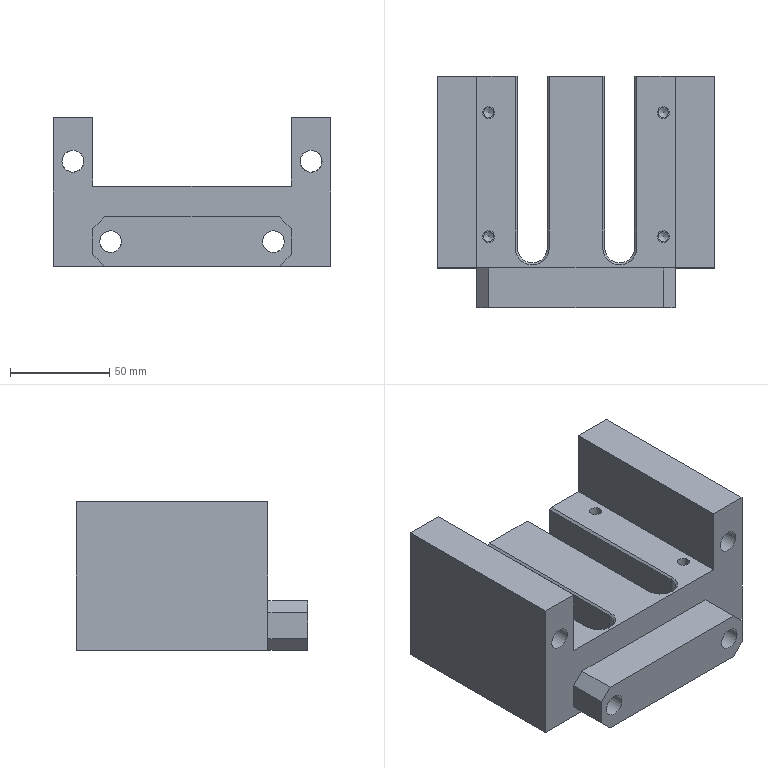Part | NX | features solid 2 | 1 solid | 58 faces | box 140 x 116.5 x 75 mm | volume 574141 mm3 | plane 36 | cylinder 14 | cone 8 | commonest cylinder face diameters 5 x4 6 x4 11 x4 15 x2
STEP:
#1=CARTESIAN_POINT('',(-13.5,271.5,-35.));
#2=VERTEX_POINT('',#1);
#3=CARTESIAN_POINT('',(13.5,271.5,-35.));
#4=VERTEX_POINT('',#3);
#5=CARTESIAN_POINT('',(0.,271.5,-35.));
#6=DIRECTION('',(1.,0.,0.));
#7=VECTOR('',#6,1000.);
#8=LINE('',#5,#7);
#9=EDGE_CURVE('',#2,#4,#8,.T.);
#10=ORIENTED_EDGE('',*,*,#9,.T.);
#11=CARTESIAN_POINT('',(14.5,271.5,-36.));
#12=VERTEX_POINT('',#11);
#13=CARTESIAN_POINT('',(17.,271.5,-38.5));
#14=DIRECTION('',(-0.7071,0.,0.7071));
#15=VECTOR('',#14,1000.);
#16=LINE('',#13,#15);
#17=EDGE_CURVE('',#4,#12,#16,.F.);
#18=ORIENTED_EDGE('',*,*,#17,.T.);
#19=CARTESIAN_POINT('',(14.5,271.5,-74.5));
#20=VERTEX_POINT('',#19);
#21=CARTESIAN_POINT('',(14.5,271.5,-55.5));
#22=DIRECTION('',(0.,0.,1.));
#23=VECTOR('',#22,1000.);
#24=LINE('',#21,#23);
#25=EDGE_CURVE('',#20,#12,#24,.T.);
#26=ORIENTED_EDGE('',*,*,#25,.F.);
#27=CARTESIAN_POINT('',(13.5,271.5,-75.5));
#28=VERTEX_POINT('',#27);
#29=CARTESIAN_POINT('',(16.75,271.5,-72.25));
#30=DIRECTION('',(-0.7071,0.,-0.7071));
#31=VECTOR('',#30,1000.);
#32=LINE('',#29,#31);
#33=EDGE_CURVE('',#20,#28,#32,.T.);
#34=ORIENTED_EDGE('',*,*,#33,.T.);
#35=CARTESIAN_POINT('',(-13.5,271.5,-75.5));
#36=VERTEX_POINT('',#35);
#37=CARTESIAN_POINT('',(0.,271.5,-75.5));
#38=DIRECTION('',(1.,0.,0.));
#39=VECTOR('',#38,1000.);
#40=LINE('',#37,#39);
#41=EDGE_CURVE('',#36,#28,#40,.T.);
#42=ORIENTED_EDGE('',*,*,#41,.F.);
#43=CARTESIAN_POINT('',(-14.5,271.5,-74.5));
#44=VERTEX_POINT('',#43);
#45=CARTESIAN_POINT('',(-16.75,271.5,-72.25));
#46=DIRECTION('',(-0.7071,0.,0.7071));
#47=VECTOR('',#46,1000.);
#48=LINE('',#45,#47);
#49=EDGE_CURVE('',#36,#44,#48,.T.);
#50=ORIENTED_EDGE('',*,*,#49,.T.);
#51=CARTESIAN_POINT('',(-14.5,271.5,-36.));
#52=VERTEX_POINT('',#51);
#53=CARTESIAN_POINT('',(-14.5,271.5,-55.5));
#54=DIRECTION('',(0.,0.,-1.));
#55=VECTOR('',#54,1000.);
#56=LINE('',#53,#55);
#57=EDGE_CURVE('',#52,#44,#56,.T.);
#58=ORIENTED_EDGE('',*,*,#57,.F.);
#59=CARTESIAN_POINT('',(-17.,271.5,-38.5));
#60=DIRECTION('',(-0.7071,0.,-0.7071));
#61=VECTOR('',#60,1000.);
#62=LINE('',#59,#61);
#63=EDGE_CURVE('',#52,#2,#62,.F.);
#64=ORIENTED_EDGE('',*,*,#63,.T.);
#65=EDGE_LOOP('',(#10,#18,#26,#34,#42,#50,#58,#64));
#66=FACE_BOUND('',#65,.T.);
#67=CARTESIAN_POINT('',(0.,271.5,-55.5));
#68=DIRECTION('',(0.,1.,0.));
#69=DIRECTION('',(0.,0.,1.));
#70=AXIS2_PLACEMENT_3D('',#67,#68,#69);
#71=PLANE('',#70);
#72=ADVANCED_FACE('',(#66),#71,.T.);
#73=CARTESIAN_POINT('',(29.5,271.5,-36.));
#74=VERTEX_POINT('',#73);
#75=CARTESIAN_POINT('',(29.5,271.5,-74.5));
#76=VERTEX_POINT('',#75);
#77=CARTESIAN_POINT('',(29.5,271.5,-55.5));
#78=DIRECTION('',(0.,0.,-1.));
#79=VECTOR('',#78,1000.);
#80=LINE('',#77,#79);
#81=EDGE_CURVE('',#74,#76,#80,.T.);
#82=ORIENTED_EDGE('',*,*,#81,.F.);
#83=CARTESIAN_POINT('',(30.5,271.5,-35.));
#84=VERTEX_POINT('',#83);
#85=CARTESIAN_POINT('',(5.,271.5,-60.5));
#86=DIRECTION('',(-0.7071,0.,-0.7071));
#87=VECTOR('',#86,1000.);
#88=LINE('',#85,#87);
#89=EDGE_CURVE('',#74,#84,#88,.F.);
#90=ORIENTED_EDGE('',*,*,#89,.T.);
#91=CARTESIAN_POINT('',(50.,271.5,-35.));
#92=VERTEX_POINT('',#91);
#93=CARTESIAN_POINT('',(0.,271.5,-35.));
#94=DIRECTION('',(1.,0.,0.));
#95=VECTOR('',#94,1000.);
#96=LINE('',#93,#95);
#97=EDGE_CURVE('',#84,#92,#96,.T.);
#98=ORIENTED_EDGE('',*,*,#97,.T.);
#99=CARTESIAN_POINT('',(50.,271.5,-0.5));
#100=VERTEX_POINT('',#99);
#101=CARTESIAN_POINT('',(50.,271.5,-55.5));
#102=DIRECTION('',(0.,0.,1.));
#103=VECTOR('',#102,1000.);
#104=LINE('',#101,#103);
#105=EDGE_CURVE('',#92,#100,#104,.T.);
#106=ORIENTED_EDGE('',*,*,#105,.T.);
#107=CARTESIAN_POINT('',(70.,271.5,-0.5));
#108=VERTEX_POINT('',#107);
#109=CARTESIAN_POINT('',(0.,271.5,-0.5));
#110=DIRECTION('',(-1.,0.,0.));
#111=VECTOR('',#110,1000.);
#112=LINE('',#109,#111);
#113=EDGE_CURVE('',#108,#100,#112,.T.);
#114=ORIENTED_EDGE('',*,*,#113,.F.);
#115=CARTESIAN_POINT('',(70.,271.5,-75.5));
#116=VERTEX_POINT('',#115);
#117=CARTESIAN_POINT('',(70.,271.5,-55.5));
#118=DIRECTION('',(0.,0.,1.));
#119=VECTOR('',#118,1000.);
#120=LINE('',#117,#119);
#121=EDGE_CURVE('',#116,#108,#120,.T.);
#122=ORIENTED_EDGE('',*,*,#121,.F.);
#123=CARTESIAN_POINT('',(30.5,271.5,-75.5));
#124=VERTEX_POINT('',#123);
#125=CARTESIAN_POINT('',(0.,271.5,-75.5));
#126=DIRECTION('',(1.,0.,0.));
#127=VECTOR('',#126,1000.);
#128=LINE('',#125,#127);
#129=EDGE_CURVE('',#124,#116,#128,.T.);
#130=ORIENTED_EDGE('',*,*,#129,.F.);
#131=CARTESIAN_POINT('',(5.25,271.5,-50.25));
#132=DIRECTION('',(-0.7071,0.,0.7071));
#133=VECTOR('',#132,1000.);
#134=LINE('',#131,#133);
#135=EDGE_CURVE('',#124,#76,#134,.T.);
#136=ORIENTED_EDGE('',*,*,#135,.T.);
#137=EDGE_LOOP('',(#82,#90,#98,#106,#114,#122,#130,#136));
#138=FACE_BOUND('',#137,.T.);
#139=CARTESIAN_POINT('',(41.,271.5,-57.5));
#140=VERTEX_POINT('',#139);
#141=CARTESIAN_POINT('',(41.,271.5,-63.));
#142=DIRECTION('',(0.,-1.,0.));
#143=DIRECTION('',(0.,0.,1.));
#144=AXIS2_PLACEMENT_3D('',#141,#142,#143);
#145=CIRCLE('',#144,5.5);
#146=EDGE_CURVE('',#140,#140,#145,.T.);
#147=ORIENTED_EDGE('',*,*,#146,.T.);
#148=EDGE_LOOP('',(#147));
#149=FACE_BOUND('',#148,.T.);
#150=CARTESIAN_POINT('',(60.,271.5,-17.));
#151=VERTEX_POINT('',#150);
#152=CARTESIAN_POINT('',(60.,271.5,-22.5));
#153=DIRECTION('',(0.,-1.,0.));
#154=DIRECTION('',(0.,0.,1.));
#155=AXIS2_PLACEMENT_3D('',#152,#153,#154);
#156=CIRCLE('',#155,5.5);
#157=EDGE_CURVE('',#151,#151,#156,.T.);
#158=ORIENTED_EDGE('',*,*,#157,.T.);
#159=EDGE_LOOP('',(#158));
#160=FACE_BOUND('',#159,.T.);
#161=CARTESIAN_POINT('',(0.,271.5,-55.5));
#162=DIRECTION('',(0.,1.,0.));
#163=DIRECTION('',(0.,0.,1.));
#164=AXIS2_PLACEMENT_3D('',#161,#162,#163);
#165=PLANE('',#164);
#166=ADVANCED_FACE('',(#138,#149,#160),#165,.T.);
#167=CARTESIAN_POINT('',(-65.5,175.,-22.5));
#168=VERTEX_POINT('',#167);
#169=CARTESIAN_POINT('',(-60.,175.,-22.5));
#170=DIRECTION('',(0.,-1.,0.));
#171=DIRECTION('',(-1.,0.,0.));
#172=AXIS2_PLACEMENT_3D('',#169,#170,#171);
#173=CIRCLE('',#172,5.5);
#174=EDGE_CURVE('',#168,#168,#173,.T.);
#175=ORIENTED_EDGE('',*,*,#174,.F.);
#176=EDGE_LOOP('',(#175));
#177=FACE_BOUND('',#176,.T.);
#178=CARTESIAN_POINT('',(70.,175.,-75.5));
#179=VERTEX_POINT('',#178);
#180=CARTESIAN_POINT('',(44.,175.,-75.5));
#181=VERTEX_POINT('',#180);
#182=CARTESIAN_POINT('',(0.,175.,-75.5));
#183=DIRECTION('',(1.,0.,0.));
#184=VECTOR('',#183,1000.);
#185=LINE('',#182,#184);
#186=EDGE_CURVE('',#179,#181,#185,.F.);
#187=ORIENTED_EDGE('',*,*,#186,.F.);
#188=CARTESIAN_POINT('',(70.,175.,-0.5));
#189=VERTEX_POINT('',#188);
#190=CARTESIAN_POINT('',(70.,175.,-55.5));
#191=DIRECTION('',(0.,0.,-1.));
#192=VECTOR('',#191,1000.);
#193=LINE('',#190,#192);
#194=EDGE_CURVE('',#179,#189,#193,.F.);
#195=ORIENTED_EDGE('',*,*,#194,.T.);
#196=CARTESIAN_POINT('',(50.,175.,-0.5));
#197=VERTEX_POINT('',#196);
#198=CARTESIAN_POINT('',(0.,175.,-0.5));
#199=DIRECTION('',(1.,0.,0.));
#200=VECTOR('',#199,1000.);
#201=LINE('',#198,#200);
#202=EDGE_CURVE('',#197,#189,#201,.T.);
#203=ORIENTED_EDGE('',*,*,#202,.F.);
#204=CARTESIAN_POINT('',(50.,175.,-35.));
#205=VERTEX_POINT('',#204);
#206=CARTESIAN_POINT('',(50.,175.,-110.5));
#207=DIRECTION('',(0.,0.,1.));
#208=VECTOR('',#207,1000.);
#209=LINE('',#206,#208);
#210=EDGE_CURVE('',#197,#205,#209,.F.);
#211=ORIENTED_EDGE('',*,*,#210,.T.);
#212=CARTESIAN_POINT('',(-50.,175.,-35.));
#213=VERTEX_POINT('',#212);
#214=CARTESIAN_POINT('',(0.,175.,-35.));
#215=DIRECTION('',(1.,0.,0.));
#216=VECTOR('',#215,1000.);
#217=LINE('',#214,#216);
#218=EDGE_CURVE('',#205,#213,#217,.F.);
#219=ORIENTED_EDGE('',*,*,#218,.T.);
#220=CARTESIAN_POINT('',(-50.,175.,-0.5));
#221=VERTEX_POINT('',#220);
#222=CARTESIAN_POINT('',(-50.,175.,-110.5));
#223=DIRECTION('',(0.,0.,-1.));
#224=VECTOR('',#223,1000.);
#225=LINE('',#222,#224);
#226=EDGE_CURVE('',#213,#221,#225,.F.);
#227=ORIENTED_EDGE('',*,*,#226,.T.);
#228=CARTESIAN_POINT('',(-70.,175.,-0.5));
#229=VERTEX_POINT('',#228);
#230=CARTESIAN_POINT('',(0.,175.,-0.5));
#231=DIRECTION('',(1.,0.,0.));
#232=VECTOR('',#231,1000.);
#233=LINE('',#230,#232);
#234=EDGE_CURVE('',#229,#221,#233,.T.);
#235=ORIENTED_EDGE('',*,*,#234,.F.);
#236=CARTESIAN_POINT('',(-70.,175.,-75.5));
#237=VERTEX_POINT('',#236);
#238=CARTESIAN_POINT('',(-70.,175.,-110.5));
#239=DIRECTION('',(0.,0.,-1.));
#240=VECTOR('',#239,1000.);
#241=LINE('',#238,#240);
#242=EDGE_CURVE('',#237,#229,#241,.F.);
#243=ORIENTED_EDGE('',*,*,#242,.F.);
#244=CARTESIAN_POINT('',(-44.,175.,-75.5));
#245=VERTEX_POINT('',#244);
#246=CARTESIAN_POINT('',(0.,175.,-75.5));
#247=DIRECTION('',(1.,0.,0.));
#248=VECTOR('',#247,1000.);
#249=LINE('',#246,#248);
#250=EDGE_CURVE('',#245,#237,#249,.F.);
#251=ORIENTED_EDGE('',*,*,#250,.F.);
#252=CARTESIAN_POINT('',(-50.,175.,-69.5));
#253=VERTEX_POINT('',#252);
#254=CARTESIAN_POINT('',(-50.,175.,-69.5));
#255=DIRECTION('',(0.7071,0.,-0.7071));
#256=VECTOR('',#255,1000.);
#257=LINE('',#254,#256);
#258=EDGE_CURVE('',#253,#245,#257,.T.);
#259=ORIENTED_EDGE('',*,*,#258,.F.);
#260=CARTESIAN_POINT('',(-50.,175.,-56.5));
#261=VERTEX_POINT('',#260);
#262=CARTESIAN_POINT('',(-50.,175.,-70.5));
#263=DIRECTION('',(0.,0.,1.));
#264=VECTOR('',#263,1000.);
#265=LINE('',#262,#264);
#266=EDGE_CURVE('',#253,#261,#265,.T.);
#267=ORIENTED_EDGE('',*,*,#266,.T.);
#268=CARTESIAN_POINT('',(-44.,175.,-50.5));
#269=VERTEX_POINT('',#268);
#270=CARTESIAN_POINT('',(-50.,175.,-56.5));
#271=DIRECTION('',(-0.7071,0.,-0.7071));
#272=VECTOR('',#271,1000.);
#273=LINE('',#270,#272);
#274=EDGE_CURVE('',#269,#261,#273,.T.);
#275=ORIENTED_EDGE('',*,*,#274,.F.);
#276=CARTESIAN_POINT('',(44.,175.,-50.5));
#277=VERTEX_POINT('',#276);
#278=CARTESIAN_POINT('',(0.,175.,-50.5));
#279=DIRECTION('',(-1.,0.,0.));
#280=VECTOR('',#279,1000.);
#281=LINE('',#278,#280);
#282=EDGE_CURVE('',#277,#269,#281,.T.);
#283=ORIENTED_EDGE('',*,*,#282,.F.);
#284=CARTESIAN_POINT('',(50.,175.,-56.5));
#285=VERTEX_POINT('',#284);
#286=CARTESIAN_POINT('',(50.,175.,-56.5));
#287=DIRECTION('',(-0.7071,0.,0.7071));
#288=VECTOR('',#287,1000.);
#289=LINE('',#286,#288);
#290=EDGE_CURVE('',#285,#277,#289,.T.);
#291=ORIENTED_EDGE('',*,*,#290,.F.);
#292=CARTESIAN_POINT('',(50.,175.,-69.5));
#293=VERTEX_POINT('',#292);
#294=CARTESIAN_POINT('',(50.,175.,-70.5));
#295=DIRECTION('',(0.,0.,1.));
#296=VECTOR('',#295,1000.);
#297=LINE('',#294,#296);
#298=EDGE_CURVE('',#293,#285,#297,.T.);
#299=ORIENTED_EDGE('',*,*,#298,.F.);
#300=CARTESIAN_POINT('',(50.,175.,-69.5));
#301=DIRECTION('',(0.7071,0.,0.7071));
#302=VECTOR('',#301,1000.);
#303=LINE('',#300,#302);
#304=EDGE_CURVE('',#181,#293,#303,.T.);
#305=ORIENTED_EDGE('',*,*,#304,.F.);
#306=EDGE_LOOP('',(#187,#195,#203,#211,#219,#227,#235,#243,#251,#259,#267,#275,#283,#291,#299,#305));
#307=FACE_BOUND('',#306,.T.);
#308=CARTESIAN_POINT('',(54.5,175.,-22.5));
#309=VERTEX_POINT('',#308);
#310=CARTESIAN_POINT('',(60.,175.,-22.5));
#311=DIRECTION('',(0.,-1.,0.));
#312=DIRECTION('',(-1.,0.,0.));
#313=AXIS2_PLACEMENT_3D('',#310,#311,#312);
#314=CIRCLE('',#313,5.5);
#315=EDGE_CURVE('',#309,#309,#314,.T.);
#316=ORIENTED_EDGE('',*,*,#315,.F.);
#317=EDGE_LOOP('',(#316));
#318=FACE_BOUND('',#317,.T.);
#319=CARTESIAN_POINT('',(0.,175.,-110.5));
#320=DIRECTION('',(0.,1.,0.));
#321=DIRECTION('',(0.,0.,1.));
#322=AXIS2_PLACEMENT_3D('',#319,#320,#321);
#323=PLANE('',#322);
#324=ADVANCED_FACE('',(#177,#307,#318),#323,.F.);
#325=CARTESIAN_POINT('',(-46.5,155.,-63.));
#326=VERTEX_POINT('',#325);
#327=CARTESIAN_POINT('',(-41.,155.,-63.));
#328=DIRECTION('',(0.,-1.,0.));
#329=DIRECTION('',(-1.,0.,0.));
#330=AXIS2_PLACEMENT_3D('',#327,#328,#329);
#331=CIRCLE('',#330,5.5);
#332=EDGE_CURVE('',#326,#326,#331,.T.);
#333=ORIENTED_EDGE('',*,*,#332,.F.);
#334=EDGE_LOOP('',(#333));
#335=FACE_BOUND('',#334,.T.);
#336=CARTESIAN_POINT('',(50.,155.,-69.5));
#337=VERTEX_POINT('',#336);
#338=CARTESIAN_POINT('',(50.,155.,-56.5));
#339=VERTEX_POINT('',#338);
#340=CARTESIAN_POINT('',(50.,155.,-70.5));
#341=DIRECTION('',(0.,0.,1.));
#342=VECTOR('',#341,1000.);
#343=LINE('',#340,#342);
#344=EDGE_CURVE('',#337,#339,#343,.T.);
#345=ORIENTED_EDGE('',*,*,#344,.T.);
#346=CARTESIAN_POINT('',(44.,155.,-50.5));
#347=VERTEX_POINT('',#346);
#348=CARTESIAN_POINT('',(32.,155.,-38.5));
#349=DIRECTION('',(-0.7071,0.,0.7071));
#350=VECTOR('',#349,1000.);
#351=LINE('',#348,#350);
#352=EDGE_CURVE('',#347,#339,#351,.F.);
#353=ORIENTED_EDGE('',*,*,#352,.F.);
#354=CARTESIAN_POINT('',(-44.,155.,-50.5));
#355=VERTEX_POINT('',#354);
#356=CARTESIAN_POINT('',(0.,155.,-50.5));
#357=DIRECTION('',(1.,0.,0.));
#358=VECTOR('',#357,1000.);
#359=LINE('',#356,#358);
#360=EDGE_CURVE('',#355,#347,#359,.T.);
#361=ORIENTED_EDGE('',*,*,#360,.F.);
#362=CARTESIAN_POINT('',(-50.,155.,-56.5));
#363=VERTEX_POINT('',#362);
#364=CARTESIAN_POINT('',(-32.,155.,-38.5));
#365=DIRECTION('',(-0.7071,0.,-0.7071));
#366=VECTOR('',#365,1000.);
#367=LINE('',#364,#366);
#368=EDGE_CURVE('',#363,#355,#367,.F.);
#369=ORIENTED_EDGE('',*,*,#368,.F.);
#370=CARTESIAN_POINT('',(-50.,155.,-69.5));
#371=VERTEX_POINT('',#370);
#372=CARTESIAN_POINT('',(-50.,155.,-70.5));
#373=DIRECTION('',(0.,0.,1.));
#374=VECTOR('',#373,1000.);
#375=LINE('',#372,#374);
#376=EDGE_CURVE('',#371,#363,#375,.T.);
#377=ORIENTED_EDGE('',*,*,#376,.F.);
#378=CARTESIAN_POINT('',(-44.,155.,-75.5));
#379=VERTEX_POINT('',#378);
#380=CARTESIAN_POINT('',(-24.5,155.,-95.));
#381=DIRECTION('',(0.7071,0.,-0.7071));
#382=VECTOR('',#381,1000.);
#383=LINE('',#380,#382);
#384=EDGE_CURVE('',#379,#371,#383,.F.);
#385=ORIENTED_EDGE('',*,*,#384,.F.);
#386=CARTESIAN_POINT('',(44.,155.,-75.5));
#387=VERTEX_POINT('',#386);
#388=CARTESIAN_POINT('',(0.,155.,-75.5));
#389=DIRECTION('',(-1.,0.,0.));
#390=VECTOR('',#389,1000.);
#391=LINE('',#388,#390);
#392=EDGE_CURVE('',#387,#379,#391,.T.);
#393=ORIENTED_EDGE('',*,*,#392,.F.);
#394=CARTESIAN_POINT('',(24.5,155.,-95.));
#395=DIRECTION('',(0.7071,0.,0.7071));
#396=VECTOR('',#395,1000.);
#397=LINE('',#394,#396);
#398=EDGE_CURVE('',#337,#387,#397,.F.);
#399=ORIENTED_EDGE('',*,*,#398,.F.);
#400=EDGE_LOOP('',(#345,#353,#361,#369,#377,#385,#393,#399));
#401=FACE_BOUND('',#400,.T.);
#402=CARTESIAN_POINT('',(35.5,155.,-63.));
#403=VERTEX_POINT('',#402);
#404=CARTESIAN_POINT('',(41.,155.,-63.));
#405=DIRECTION('',(0.,-1.,0.));
#406=DIRECTION('',(-1.,0.,0.));
#407=AXIS2_PLACEMENT_3D('',#404,#405,#406);
#408=CIRCLE('',#407,5.5);
#409=EDGE_CURVE('',#403,#403,#408,.T.);
#410=ORIENTED_EDGE('',*,*,#409,.F.);
#411=EDGE_LOOP('',(#410));
#412=FACE_BOUND('',#411,.T.);
#413=CARTESIAN_POINT('',(0.,155.,-70.5));
#414=DIRECTION('',(0.,-1.,0.));
#415=DIRECTION('',(0.,0.,-1.));
#416=AXIS2_PLACEMENT_3D('',#413,#414,#415);
#417=PLANE('',#416);
#418=ADVANCED_FACE('',(#335,#401,#412),#417,.T.);
#419=CARTESIAN_POINT('',(-41.,253.25,-35.));
#420=VERTEX_POINT('',#419);
#421=CARTESIAN_POINT('',(-44.,253.25,-35.));
#422=DIRECTION('',(0.,0.,1.));
#423=DIRECTION('',(1.,0.,0.));
#424=AXIS2_PLACEMENT_3D('',#421,#422,#423);
#425=CIRCLE('',#424,3.);
#426=EDGE_CURVE('',#420,#420,#425,.F.);
#427=ORIENTED_EDGE('',*,*,#426,.T.);
#428=EDGE_LOOP('',(#427));
#429=FACE_BOUND('',#428,.T.);
#430=CARTESIAN_POINT('',(47.,253.25,-35.));
#431=VERTEX_POINT('',#430);
#432=CARTESIAN_POINT('',(44.,253.25,-35.));
#433=DIRECTION('',(0.,0.,1.));
#434=DIRECTION('',(1.,0.,0.));
#435=AXIS2_PLACEMENT_3D('',#432,#433,#434);
#436=CIRCLE('',#435,3.);
#437=EDGE_CURVE('',#431,#431,#436,.T.);
#438=ORIENTED_EDGE('',*,*,#437,.F.);
#439=EDGE_LOOP('',(#438));
#440=FACE_BOUND('',#439,.T.);
#441=ORIENTED_EDGE('',*,*,#97,.F.);
#442=CARTESIAN_POINT('',(30.5,185.,-35.));
#443=VERTEX_POINT('',#442);
#444=CARTESIAN_POINT('',(30.5,155.,-35.));
#445=DIRECTION('',(0.,-1.,0.));
#446=VECTOR('',#445,1000.);
#447=LINE('',#444,#446);
#448=EDGE_CURVE('',#84,#443,#447,.T.);
#449=ORIENTED_EDGE('',*,*,#448,.T.);
#450=CARTESIAN_POINT('',(13.5,185.,-35.));
#451=VERTEX_POINT('',#450);
#452=CARTESIAN_POINT('',(22.,185.,-35.));
#453=DIRECTION('',(0.,0.,-1.));
#454=DIRECTION('',(1.,0.,0.));
#455=AXIS2_PLACEMENT_3D('',#452,#453,#454);
#456=CIRCLE('',#455,8.5);
#457=EDGE_CURVE('',#443,#451,#456,.T.);
#458=ORIENTED_EDGE('',*,*,#457,.T.);
#459=CARTESIAN_POINT('',(13.5,155.,-35.));
#460=DIRECTION('',(0.,1.,0.));
#461=VECTOR('',#460,1000.);
#462=LINE('',#459,#461);
#463=EDGE_CURVE('',#451,#4,#462,.T.);
#464=ORIENTED_EDGE('',*,*,#463,.T.);
#465=ORIENTED_EDGE('',*,*,#9,.F.);
#466=CARTESIAN_POINT('',(-13.5,185.,-35.));
#467=VERTEX_POINT('',#466);
#468=CARTESIAN_POINT('',(-13.5,155.,-35.));
#469=DIRECTION('',(0.,-1.,0.));
#470=VECTOR('',#469,1000.);
#471=LINE('',#468,#470);
#472=EDGE_CURVE('',#2,#467,#471,.T.);
#473=ORIENTED_EDGE('',*,*,#472,.T.);
#474=CARTESIAN_POINT('',(-30.5,185.,-35.));
#475=VERTEX_POINT('',#474);
#476=CARTESIAN_POINT('',(-22.,185.,-35.));
#477=DIRECTION('',(0.,0.,-1.));
#478=DIRECTION('',(1.,0.,0.));
#479=AXIS2_PLACEMENT_3D('',#476,#477,#478);
#480=CIRCLE('',#479,8.5);
#481=EDGE_CURVE('',#467,#475,#480,.T.);
#482=ORIENTED_EDGE('',*,*,#481,.T.);
#483=CARTESIAN_POINT('',(-30.5,271.5,-35.));
#484=VERTEX_POINT('',#483);
#485=CARTESIAN_POINT('',(-30.5,155.,-35.));
#486=DIRECTION('',(0.,1.,0.));
#487=VECTOR('',#486,1000.);
#488=LINE('',#485,#487);
#489=EDGE_CURVE('',#475,#484,#488,.T.);
#490=ORIENTED_EDGE('',*,*,#489,.T.);
#491=CARTESIAN_POINT('',(-50.,271.5,-35.));
#492=VERTEX_POINT('',#491);
#493=CARTESIAN_POINT('',(0.,271.5,-35.));
#494=DIRECTION('',(1.,0.,0.));
#495=VECTOR('',#494,1000.);
#496=LINE('',#493,#495);
#497=EDGE_CURVE('',#492,#484,#496,.T.);
#498=ORIENTED_EDGE('',*,*,#497,.F.);
#499=CARTESIAN_POINT('',(-50.,155.,-35.));
#500=DIRECTION('',(0.,-1.,0.));
#501=VECTOR('',#500,1000.);
#502=LINE('',#499,#501);
#503=EDGE_CURVE('',#492,#213,#502,.T.);
#504=ORIENTED_EDGE('',*,*,#503,.T.);
#505=ORIENTED_EDGE('',*,*,#218,.F.);
#506=CARTESIAN_POINT('',(50.,155.,-35.));
#507=DIRECTION('',(0.,1.,0.));
#508=VECTOR('',#507,1000.);
#509=LINE('',#506,#508);
#510=EDGE_CURVE('',#205,#92,#509,.T.);
#511=ORIENTED_EDGE('',*,*,#510,.T.);
#512=EDGE_LOOP('',(#441,#449,#458,#464,#465,#473,#482,#490,#498,#504,#505,#511));
#513=FACE_BOUND('',#512,.T.);
#514=CARTESIAN_POINT('',(47.,190.75,-35.));
#515=VERTEX_POINT('',#514);
#516=CARTESIAN_POINT('',(44.,190.75,-35.));
#517=DIRECTION('',(0.,0.,1.));
#518=DIRECTION('',(1.,0.,0.));
#519=AXIS2_PLACEMENT_3D('',#516,#517,#518);
#520=CIRCLE('',#519,3.);
#521=EDGE_CURVE('',#515,#515,#520,.T.);
#522=ORIENTED_EDGE('',*,*,#521,.F.);
#523=EDGE_LOOP('',(#522));
#524=FACE_BOUND('',#523,.T.);
#525=CARTESIAN_POINT('',(-41.,190.75,-35.));
#526=VERTEX_POINT('',#525);
#527=CARTESIAN_POINT('',(-44.,190.75,-35.));
#528=DIRECTION('',(0.,0.,1.));
#529=DIRECTION('',(1.,0.,0.));
#530=AXIS2_PLACEMENT_3D('',#527,#528,#529);
#531=CIRCLE('',#530,3.);
#532=EDGE_CURVE('',#526,#526,#531,.F.);
#533=ORIENTED_EDGE('',*,*,#532,.T.);
#534=EDGE_LOOP('',(#533));
#535=FACE_BOUND('',#534,.T.);
#536=CARTESIAN_POINT('',(-11.5,155.,-35.));
#537=DIRECTION('',(0.,0.,-1.));
#538=DIRECTION('',(0.,1.,0.));
#539=AXIS2_PLACEMENT_3D('',#536,#537,#538);
#540=PLANE('',#539);
#541=ADVANCED_FACE('',(#429,#440,#513,#524,#535),#540,.F.);
#542=ORIENTED_EDGE('',*,*,#194,.F.);
#543=CARTESIAN_POINT('',(70.,245.25,-75.5));
#544=DIRECTION('',(0.,-1.,0.));
#545=VECTOR('',#544,1000.);
#546=LINE('',#543,#545);
#547=EDGE_CURVE('',#116,#179,#546,.T.);
#548=ORIENTED_EDGE('',*,*,#547,.F.);
#549=ORIENTED_EDGE('',*,*,#121,.T.);
#550=CARTESIAN_POINT('',(70.,223.25,-0.5));
#551=DIRECTION('',(0.,1.,0.));
#552=VECTOR('',#551,1000.);
#553=LINE('',#550,#552);
#554=EDGE_CURVE('',#189,#108,#553,.T.);
#555=ORIENTED_EDGE('',*,*,#554,.F.);
#556=EDGE_LOOP('',(#542,#548,#549,#555));
#557=FACE_BOUND('',#556,.T.);
#558=CARTESIAN_POINT('',(70.,245.25,-55.5));
#559=DIRECTION('',(1.,0.,0.));
#560=DIRECTION('',(0.,0.,1.));
#561=AXIS2_PLACEMENT_3D('',#558,#559,#560);
#562=PLANE('',#561);
#563=ADVANCED_FACE('',(#557),#562,.T.);
#564=ORIENTED_EDGE('',*,*,#497,.T.);
#565=CARTESIAN_POINT('',(-29.5,271.5,-36.));
#566=VERTEX_POINT('',#565);
#567=CARTESIAN_POINT('',(-5.,271.5,-60.5));
#568=DIRECTION('',(-0.7071,0.,0.7071));
#569=VECTOR('',#568,1000.);
#570=LINE('',#567,#569);
#571=EDGE_CURVE('',#484,#566,#570,.F.);
#572=ORIENTED_EDGE('',*,*,#571,.T.);
#573=CARTESIAN_POINT('',(-29.5,271.5,-74.5));
#574=VERTEX_POINT('',#573);
#575=CARTESIAN_POINT('',(-29.5,271.5,-55.5));
#576=DIRECTION('',(0.,0.,1.));
#577=VECTOR('',#576,1000.);
#578=LINE('',#575,#577);
#579=EDGE_CURVE('',#574,#566,#578,.T.);
#580=ORIENTED_EDGE('',*,*,#579,.F.);
#581=CARTESIAN_POINT('',(-30.5,271.5,-75.5));
#582=VERTEX_POINT('',#581);
#583=CARTESIAN_POINT('',(-5.25,271.5,-50.25));
#584=DIRECTION('',(-0.7071,0.,-0.7071));
#585=VECTOR('',#584,1000.);
#586=LINE('',#583,#585);
#587=EDGE_CURVE('',#574,#582,#586,.T.);
#588=ORIENTED_EDGE('',*,*,#587,.T.);
#589=CARTESIAN_POINT('',(-70.,271.5,-75.5));
#590=VERTEX_POINT('',#589);
#591=CARTESIAN_POINT('',(0.,271.5,-75.5));
#592=DIRECTION('',(1.,0.,0.));
#593=VECTOR('',#592,1000.);
#594=LINE('',#591,#593);
#595=EDGE_CURVE('',#590,#582,#594,.T.);
#596=ORIENTED_EDGE('',*,*,#595,.F.);
#597=CARTESIAN_POINT('',(-70.,271.5,-0.5));
#598=VERTEX_POINT('',#597);
#599=CARTESIAN_POINT('',(-70.,271.5,-55.5));
#600=DIRECTION('',(0.,0.,1.));
#601=VECTOR('',#600,1000.);
#602=LINE('',#599,#601);
#603=EDGE_CURVE('',#590,#598,#602,.T.);
#604=ORIENTED_EDGE('',*,*,#603,.T.);
#605=CARTESIAN_POINT('',(-50.,271.5,-0.5));
#606=VERTEX_POINT('',#605);
#607=CARTESIAN_POINT('',(0.,271.5,-0.5));
#608=DIRECTION('',(-1.,0.,0.));
#609=VECTOR('',#608,1000.);
#610=LINE('',#607,#609);
#611=EDGE_CURVE('',#606,#598,#610,.T.);
#612=ORIENTED_EDGE('',*,*,#611,.F.);
#613=CARTESIAN_POINT('',(-50.,271.5,-25.5));
#614=DIRECTION('',(0.,0.,1.));
#615=VECTOR('',#614,1000.);
#616=LINE('',#613,#615);
#617=EDGE_CURVE('',#492,#606,#616,.T.);
#618=ORIENTED_EDGE('',*,*,#617,.F.);
#619=EDGE_LOOP('',(#564,#572,#580,#588,#596,#604,#612,#618));
#620=FACE_BOUND('',#619,.T.);
#621=CARTESIAN_POINT('',(-60.,271.5,-17.));
#622=VERTEX_POINT('',#621);
#623=CARTESIAN_POINT('',(-60.,271.5,-22.5));
#624=DIRECTION('',(0.,-1.,0.));
#625=DIRECTION('',(0.,0.,1.));
#626=AXIS2_PLACEMENT_3D('',#623,#624,#625);
#627=CIRCLE('',#626,5.5);
#628=EDGE_CURVE('',#622,#622,#627,.T.);
#629=ORIENTED_EDGE('',*,*,#628,.T.);
#630=EDGE_LOOP('',(#629));
#631=FACE_BOUND('',#630,.T.);
#632=CARTESIAN_POINT('',(-41.,271.5,-57.5));
#633=VERTEX_POINT('',#632);
#634=CARTESIAN_POINT('',(-41.,271.5,-63.));
#635=DIRECTION('',(0.,-1.,0.));
#636=DIRECTION('',(0.,0.,1.));
#637=AXIS2_PLACEMENT_3D('',#634,#635,#636);
#638=CIRCLE('',#637,5.5);
#639=EDGE_CURVE('',#633,#633,#638,.T.);
#640=ORIENTED_EDGE('',*,*,#639,.T.);
#641=EDGE_LOOP('',(#640));
#642=FACE_BOUND('',#641,.T.);
#643=CARTESIAN_POINT('',(0.,271.5,-55.5));
#644=DIRECTION('',(0.,1.,0.));
#645=DIRECTION('',(0.,0.,1.));
#646=AXIS2_PLACEMENT_3D('',#643,#644,#645);
#647=PLANE('',#646);
#648=ADVANCED_FACE('',(#620,#631,#642),#647,.T.);
#649=ORIENTED_EDGE('',*,*,#603,.F.);
#650=CARTESIAN_POINT('',(-70.,245.25,-75.5));
#651=DIRECTION('',(0.,1.,0.));
#652=VECTOR('',#651,1000.);
#653=LINE('',#650,#652);
#654=EDGE_CURVE('',#237,#590,#653,.T.);
#655=ORIENTED_EDGE('',*,*,#654,.F.);
#656=ORIENTED_EDGE('',*,*,#242,.T.);
#657=CARTESIAN_POINT('',(-70.,223.25,-0.5));
#658=DIRECTION('',(0.,-1.,0.));
#659=VECTOR('',#658,1000.);
#660=LINE('',#657,#659);
#661=EDGE_CURVE('',#598,#229,#660,.T.);
#662=ORIENTED_EDGE('',*,*,#661,.F.);
#663=EDGE_LOOP('',(#649,#655,#656,#662));
#664=FACE_BOUND('',#663,.T.);
#665=CARTESIAN_POINT('',(-70.,245.25,-55.5));
#666=DIRECTION('',(-1.,0.,0.));
#667=DIRECTION('',(0.,0.,-1.));
#668=AXIS2_PLACEMENT_3D('',#665,#666,#667);
#669=PLANE('',#668);
#670=ADVANCED_FACE('',(#664),#669,.T.);
#671=ORIENTED_EDGE('',*,*,#595,.T.);
#672=CARTESIAN_POINT('',(-30.5,185.,-75.5));
#673=VERTEX_POINT('',#672);
#674=CARTESIAN_POINT('',(-30.5,185.,-75.5));
#675=DIRECTION('',(0.,-1.,0.));
#676=VECTOR('',#675,1000.);
#677=LINE('',#674,#676);
#678=EDGE_CURVE('',#582,#673,#677,.T.);
#679=ORIENTED_EDGE('',*,*,#678,.T.);
#680=CARTESIAN_POINT('',(-13.5,185.,-75.5));
#681=VERTEX_POINT('',#680);
#682=CARTESIAN_POINT('',(-22.,185.,-75.5));
#683=DIRECTION('',(0.,0.,-1.));
#684=DIRECTION('',(1.,0.,0.));
#685=AXIS2_PLACEMENT_3D('',#682,#683,#684);
#686=CIRCLE('',#685,8.5);
#687=EDGE_CURVE('',#673,#681,#686,.F.);
#688=ORIENTED_EDGE('',*,*,#687,.T.);
#689=CARTESIAN_POINT('',(-13.5,271.5,-75.5));
#690=DIRECTION('',(0.,1.,0.));
#691=VECTOR('',#690,1000.);
#692=LINE('',#689,#691);
#693=EDGE_CURVE('',#681,#36,#692,.T.);
#694=ORIENTED_EDGE('',*,*,#693,.T.);
#695=ORIENTED_EDGE('',*,*,#41,.T.);
#696=CARTESIAN_POINT('',(13.5,185.,-75.5));
#697=VERTEX_POINT('',#696);
#698=CARTESIAN_POINT('',(13.5,185.,-75.5));
#699=DIRECTION('',(0.,-1.,0.));
#700=VECTOR('',#699,1000.);
#701=LINE('',#698,#700);
#702=EDGE_CURVE('',#28,#697,#701,.T.);
#703=ORIENTED_EDGE('',*,*,#702,.T.);
#704=CARTESIAN_POINT('',(30.5,185.,-75.5));
#705=VERTEX_POINT('',#704);
#706=CARTESIAN_POINT('',(22.,185.,-75.5));
#707=DIRECTION('',(0.,0.,-1.));
#708=DIRECTION('',(1.,0.,0.));
#709=AXIS2_PLACEMENT_3D('',#706,#707,#708);
#710=CIRCLE('',#709,8.5);
#711=EDGE_CURVE('',#697,#705,#710,.F.);
#712=ORIENTED_EDGE('',*,*,#711,.T.);
#713=CARTESIAN_POINT('',(30.5,271.5,-75.5));
#714=DIRECTION('',(0.,1.,0.));
#715=VECTOR('',#714,1000.);
#716=LINE('',#713,#715);
#717=EDGE_CURVE('',#705,#124,#716,.T.);
#718=ORIENTED_EDGE('',*,*,#717,.T.);
#719=ORIENTED_EDGE('',*,*,#129,.T.);
#720=ORIENTED_EDGE('',*,*,#547,.T.);
#721=ORIENTED_EDGE('',*,*,#186,.T.);
#722=CARTESIAN_POINT('',(44.,245.25,-75.5));
#723=DIRECTION('',(0.,1.,0.));
#724=VECTOR('',#723,1000.);
#725=LINE('',#722,#724);
#726=EDGE_CURVE('',#387,#181,#725,.T.);
#727=ORIENTED_EDGE('',*,*,#726,.F.);
#728=ORIENTED_EDGE('',*,*,#392,.T.);
#729=CARTESIAN_POINT('',(-44.,245.25,-75.5));
#730=DIRECTION('',(0.,-1.,0.));
#731=VECTOR('',#730,1000.);
#732=LINE('',#729,#731);
#733=EDGE_CURVE('',#245,#379,#732,.T.);
#734=ORIENTED_EDGE('',*,*,#733,.F.);
#735=ORIENTED_EDGE('',*,*,#250,.T.);
#736=ORIENTED_EDGE('',*,*,#654,.T.);
#737=EDGE_LOOP('',(#671,#679,#688,#694,#695,#703,#712,#718,#719,#720,#721,#727,#728,#734,#735,#736));
#738=FACE_BOUND('',#737,.T.);
#739=CARTESIAN_POINT('',(0.,245.25,-75.5));
#740=DIRECTION('',(0.,0.,-1.));
#741=DIRECTION('',(1.,0.,0.));
#742=AXIS2_PLACEMENT_3D('',#739,#740,#741);
#743=PLANE('',#742);
#744=ADVANCED_FACE('',(#738),#743,.T.);
#745=ORIENTED_EDGE('',*,*,#611,.T.);
#746=ORIENTED_EDGE('',*,*,#661,.T.);
#747=ORIENTED_EDGE('',*,*,#234,.T.);
#748=CARTESIAN_POINT('',(-50.,155.,-0.5));
#749=DIRECTION('',(0.,-1.,0.));
#750=VECTOR('',#749,1000.);
#751=LINE('',#748,#750);
#752=EDGE_CURVE('',#606,#221,#751,.T.);
#753=ORIENTED_EDGE('',*,*,#752,.F.);
#754=EDGE_LOOP('',(#745,#746,#747,#753));
#755=FACE_BOUND('',#754,.T.);
#756=CARTESIAN_POINT('',(-11.5,155.,-0.5));
#757=DIRECTION('',(0.,0.,1.));
#758=DIRECTION('',(0.,-1.,0.));
#759=AXIS2_PLACEMENT_3D('',#756,#757,#758);
#760=PLANE('',#759);
#761=ADVANCED_FACE('',(#755),#760,.T.);
#762=ORIENTED_EDGE('',*,*,#226,.F.);
#763=ORIENTED_EDGE('',*,*,#503,.F.);
#764=ORIENTED_EDGE('',*,*,#617,.T.);
#765=ORIENTED_EDGE('',*,*,#752,.T.);
#766=EDGE_LOOP('',(#762,#763,#764,#765));
#767=FACE_BOUND('',#766,.T.);
#768=CARTESIAN_POINT('',(-50.,155.,-25.5));
#769=DIRECTION('',(-1.,0.,0.));
#770=DIRECTION('',(0.,0.,-1.));
#771=AXIS2_PLACEMENT_3D('',#768,#769,#770);
#772=PLANE('',#771);
#773=ADVANCED_FACE('',(#767),#772,.F.);
#774=CARTESIAN_POINT('',(50.,155.,-0.5));
#775=DIRECTION('',(0.,-1.,0.));
#776=VECTOR('',#775,1000.);
#777=LINE('',#774,#776);
#778=EDGE_CURVE('',#100,#197,#777,.T.);
#779=ORIENTED_EDGE('',*,*,#778,.T.);
#780=ORIENTED_EDGE('',*,*,#202,.T.);
#781=ORIENTED_EDGE('',*,*,#554,.T.);
#782=ORIENTED_EDGE('',*,*,#113,.T.);
#783=EDGE_LOOP('',(#779,#780,#781,#782));
#784=FACE_BOUND('',#783,.T.);
#785=CARTESIAN_POINT('',(-11.5,155.,-0.5));
#786=DIRECTION('',(0.,0.,1.));
#787=DIRECTION('',(0.,-1.,0.));
#788=AXIS2_PLACEMENT_3D('',#785,#786,#787);
#789=PLANE('',#788);
#790=ADVANCED_FACE('',(#784),#789,.T.);
#791=ORIENTED_EDGE('',*,*,#210,.F.);
#792=ORIENTED_EDGE('',*,*,#778,.F.);
#793=ORIENTED_EDGE('',*,*,#105,.F.);
#794=ORIENTED_EDGE('',*,*,#510,.F.);
#795=EDGE_LOOP('',(#791,#792,#793,#794));
#796=FACE_BOUND('',#795,.T.);
#797=CARTESIAN_POINT('',(50.,155.,-25.5));
#798=DIRECTION('',(1.,0.,0.));
#799=DIRECTION('',(0.,0.,-1.));
#800=AXIS2_PLACEMENT_3D('',#797,#798,#799);
#801=PLANE('',#800);
#802=ADVANCED_FACE('',(#796),#801,.F.);
#803=ORIENTED_EDGE('',*,*,#282,.T.);
#804=CARTESIAN_POINT('',(-44.,162.5,-50.5));
#805=DIRECTION('',(0.,1.,0.));
#806=VECTOR('',#805,1000.);
#807=LINE('',#804,#806);
#808=EDGE_CURVE('',#355,#269,#807,.T.);
#809=ORIENTED_EDGE('',*,*,#808,.F.);
#810=ORIENTED_EDGE('',*,*,#360,.T.);
#811=CARTESIAN_POINT('',(44.,162.5,-50.5));
#812=DIRECTION('',(0.,-1.,0.));
#813=VECTOR('',#812,1000.);
#814=LINE('',#811,#813);
#815=EDGE_CURVE('',#277,#347,#814,.T.);
#816=ORIENTED_EDGE('',*,*,#815,.F.);
#817=EDGE_LOOP('',(#803,#809,#810,#816));
#818=FACE_BOUND('',#817,.T.);
#819=CARTESIAN_POINT('',(0.,162.5,-50.5));
#820=DIRECTION('',(0.,0.,1.));
#821=DIRECTION('',(-1.,0.,0.));
#822=AXIS2_PLACEMENT_3D('',#819,#820,#821);
#823=PLANE('',#822);
#824=ADVANCED_FACE('',(#818),#823,.T.);
#825=ORIENTED_EDGE('',*,*,#298,.T.);
#826=CARTESIAN_POINT('',(50.,162.5,-56.5));
#827=DIRECTION('',(0.,1.,0.));
#828=VECTOR('',#827,1000.);
#829=LINE('',#826,#828);
#830=EDGE_CURVE('',#339,#285,#829,.T.);
#831=ORIENTED_EDGE('',*,*,#830,.F.);
#832=ORIENTED_EDGE('',*,*,#344,.F.);
#833=CARTESIAN_POINT('',(50.,162.5,-69.5));
#834=DIRECTION('',(0.,-1.,0.));
#835=VECTOR('',#834,1000.);
#836=LINE('',#833,#835);
#837=EDGE_CURVE('',#293,#337,#836,.T.);
#838=ORIENTED_EDGE('',*,*,#837,.F.);
#839=EDGE_LOOP('',(#825,#831,#832,#838));
#840=FACE_BOUND('',#839,.T.);
#841=CARTESIAN_POINT('',(50.,162.5,-70.5));
#842=DIRECTION('',(1.,0.,0.));
#843=DIRECTION('',(0.,0.,1.));
#844=AXIS2_PLACEMENT_3D('',#841,#842,#843);
#845=PLANE('',#844);
#846=ADVANCED_FACE('',(#840),#845,.T.);
#847=ORIENTED_EDGE('',*,*,#376,.T.);
#848=CARTESIAN_POINT('',(-50.,162.5,-56.5));
#849=DIRECTION('',(0.,-1.,0.));
#850=VECTOR('',#849,1000.);
#851=LINE('',#848,#850);
#852=EDGE_CURVE('',#261,#363,#851,.T.);
#853=ORIENTED_EDGE('',*,*,#852,.F.);
#854=ORIENTED_EDGE('',*,*,#266,.F.);
#855=CARTESIAN_POINT('',(-50.,162.5,-69.5));
#856=DIRECTION('',(0.,1.,0.));
#857=VECTOR('',#856,1000.);
#858=LINE('',#855,#857);
#859=EDGE_CURVE('',#371,#253,#858,.T.);
#860=ORIENTED_EDGE('',*,*,#859,.F.);
#861=EDGE_LOOP('',(#847,#853,#854,#860));
#862=FACE_BOUND('',#861,.T.);
#863=CARTESIAN_POINT('',(-50.,162.5,-70.5));
#864=DIRECTION('',(-1.,0.,0.));
#865=DIRECTION('',(0.,0.,-1.));
#866=AXIS2_PLACEMENT_3D('',#863,#864,#865);
#867=PLANE('',#866);
#868=ADVANCED_FACE('',(#862),#867,.T.);
#869=CARTESIAN_POINT('',(46.5,190.75,-47.5));
#870=VERTEX_POINT('',#869);
#871=CARTESIAN_POINT('',(44.,190.75,-47.5));
#872=DIRECTION('',(0.,0.,1.));
#873=DIRECTION('',(1.,0.,0.));
#874=AXIS2_PLACEMENT_3D('',#871,#872,#873);
#875=CIRCLE('',#874,2.5);
#876=EDGE_CURVE('',#870,#870,#875,.F.);
#877=ORIENTED_EDGE('',*,*,#876,.T.);
#878=EDGE_LOOP('',(#877));
#879=FACE_BOUND('',#878,.T.);
#880=CARTESIAN_POINT('',(41.,190.75,-47.5));
#881=VERTEX_POINT('',#880);
#882=CARTESIAN_POINT('',(44.,190.75,-47.5));
#883=DIRECTION('',(0.,0.,-1.));
#884=DIRECTION('',(-1.,0.,0.));
#885=AXIS2_PLACEMENT_3D('',#882,#883,#884);
#886=CIRCLE('',#885,3.);
#887=EDGE_CURVE('',#881,#881,#886,.F.);
#888=ORIENTED_EDGE('',*,*,#887,.T.);
#889=EDGE_LOOP('',(#888));
#890=FACE_BOUND('',#889,.T.);
#891=CARTESIAN_POINT('',(44.,190.75,-47.5));
#892=DIRECTION('',(0.,0.,-1.));
#893=DIRECTION('',(1.,0.,0.));
#894=AXIS2_PLACEMENT_3D('',#891,#892,#893);
#895=PLANE('',#894);
#896=ADVANCED_FACE('',(#879,#890),#895,.F.);
#897=ORIENTED_EDGE('',*,*,#887,.F.);
#898=EDGE_LOOP('',(#897));
#899=FACE_BOUND('',#898,.T.);
#900=ORIENTED_EDGE('',*,*,#521,.T.);
#901=EDGE_LOOP('',(#900));
#902=FACE_BOUND('',#901,.T.);
#903=CARTESIAN_POINT('',(44.,190.75,-35.5));
#904=DIRECTION('',(0.,0.,-1.));
#905=DIRECTION('',(-1.,0.,0.));
#906=AXIS2_PLACEMENT_3D('',#903,#904,#905);
#907=CYLINDRICAL_SURFACE('',#906,3.);
#908=ADVANCED_FACE('',(#899,#902),#907,.F.);
#909=ORIENTED_EDGE('',*,*,#876,.F.);
#910=EDGE_LOOP('',(#909));
#911=FACE_BOUND('',#910,.T.);
#912=CARTESIAN_POINT('',(41.5,190.75,-49.5));
#913=VERTEX_POINT('',#912);
#914=CARTESIAN_POINT('',(44.,190.75,-49.5));
#915=DIRECTION('',(0.,0.,1.));
#916=DIRECTION('',(-1.,0.,0.));
#917=AXIS2_PLACEMENT_3D('',#914,#915,#916);
#918=CIRCLE('',#917,2.5);
#919=EDGE_CURVE('',#913,#913,#918,.F.);
#920=ORIENTED_EDGE('',*,*,#919,.T.);
#921=EDGE_LOOP('',(#920));
#922=FACE_BOUND('',#921,.T.);
#923=CARTESIAN_POINT('',(44.,190.75,-35.5));
#924=DIRECTION('',(0.,0.,-1.));
#925=DIRECTION('',(-1.,0.,0.));
#926=AXIS2_PLACEMENT_3D('',#923,#924,#925);
#927=CYLINDRICAL_SURFACE('',#926,2.5);
#928=ADVANCED_FACE('',(#911,#922),#927,.F.);
#929=ORIENTED_EDGE('',*,*,#919,.F.);
#930=EDGE_LOOP('',(#929));
#931=FACE_BOUND('',#930,.T.);
#932=CARTESIAN_POINT('',(44.,190.75,-51.002));
#933=VERTEX_POINT('',#932);
#934=VERTEX_LOOP('',#933);
#935=FACE_BOUND('',#934,.T.);
#936=CARTESIAN_POINT('',(44.,190.75,-51.002));
#937=DIRECTION('',(0.,0.,1.));
#938=DIRECTION('',(-1.,0.,0.));
#939=AXIS2_PLACEMENT_3D('',#936,#937,#938);
#940=CONICAL_SURFACE('',#939,0.,1.03);
#941=ADVANCED_FACE('',(#931,#935),#940,.F.);
#942=CARTESIAN_POINT('',(46.5,253.25,-47.5));
#943=VERTEX_POINT('',#942);
#944=CARTESIAN_POINT('',(44.,253.25,-47.5));
#945=DIRECTION('',(0.,0.,1.));
#946=DIRECTION('',(1.,0.,0.));
#947=AXIS2_PLACEMENT_3D('',#944,#945,#946);
#948=CIRCLE('',#947,2.5);
#949=EDGE_CURVE('',#943,#943,#948,.F.);
#950=ORIENTED_EDGE('',*,*,#949,.T.);
#951=EDGE_LOOP('',(#950));
#952=FACE_BOUND('',#951,.T.);
#953=CARTESIAN_POINT('',(41.,253.25,-47.5));
#954=VERTEX_POINT('',#953);
#955=CARTESIAN_POINT('',(44.,253.25,-47.5));
#956=DIRECTION('',(0.,0.,-1.));
#957=DIRECTION('',(-1.,0.,0.));
#958=AXIS2_PLACEMENT_3D('',#955,#956,#957);
#959=CIRCLE('',#958,3.);
#960=EDGE_CURVE('',#954,#954,#959,.F.);
#961=ORIENTED_EDGE('',*,*,#960,.T.);
#962=EDGE_LOOP('',(#961));
#963=FACE_BOUND('',#962,.T.);
#964=CARTESIAN_POINT('',(44.,253.25,-47.5));
#965=DIRECTION('',(0.,0.,-1.));
#966=DIRECTION('',(1.,0.,0.));
#967=AXIS2_PLACEMENT_3D('',#964,#965,#966);
#968=PLANE('',#967);
#969=ADVANCED_FACE('',(#952,#963),#968,.F.);
#970=ORIENTED_EDGE('',*,*,#960,.F.);
#971=EDGE_LOOP('',(#970));
#972=FACE_BOUND('',#971,.T.);
#973=ORIENTED_EDGE('',*,*,#437,.T.);
#974=EDGE_LOOP('',(#973));
#975=FACE_BOUND('',#974,.T.);
#976=CARTESIAN_POINT('',(44.,253.25,-35.5));
#977=DIRECTION('',(0.,0.,-1.));
#978=DIRECTION('',(-1.,0.,0.));
#979=AXIS2_PLACEMENT_3D('',#976,#977,#978);
#980=CYLINDRICAL_SURFACE('',#979,3.);
#981=ADVANCED_FACE('',(#972,#975),#980,.F.);
#982=ORIENTED_EDGE('',*,*,#949,.F.);
#983=EDGE_LOOP('',(#982));
#984=FACE_BOUND('',#983,.T.);
#985=CARTESIAN_POINT('',(41.5,253.25,-49.5));
#986=VERTEX_POINT('',#985);
#987=CARTESIAN_POINT('',(44.,253.25,-49.5));
#988=DIRECTION('',(0.,0.,1.));
#989=DIRECTION('',(-1.,0.,0.));
#990=AXIS2_PLACEMENT_3D('',#987,#988,#989);
#991=CIRCLE('',#990,2.5);
#992=EDGE_CURVE('',#986,#986,#991,.F.);
#993=ORIENTED_EDGE('',*,*,#992,.T.);
#994=EDGE_LOOP('',(#993));
#995=FACE_BOUND('',#994,.T.);
#996=CARTESIAN_POINT('',(44.,253.25,-35.5));
#997=DIRECTION('',(0.,0.,-1.));
#998=DIRECTION('',(-1.,0.,0.));
#999=AXIS2_PLACEMENT_3D('',#996,#997,#998);
#1000=CYLINDRICAL_SURFACE('',#999,2.5);
#1001=ADVANCED_FACE('',(#984,#995),#1000,.F.);
#1002=ORIENTED_EDGE('',*,*,#992,.F.);
#1003=EDGE_LOOP('',(#1002));
#1004=FACE_BOUND('',#1003,.T.);
#1005=CARTESIAN_POINT('',(44.,253.25,-51.002));
#1006=VERTEX_POINT('',#1005);
#1007=VERTEX_LOOP('',#1006);
#1008=FACE_BOUND('',#1007,.T.);
#1009=CARTESIAN_POINT('',(44.,253.25,-51.002));
#1010=DIRECTION('',(0.,0.,1.));
#1011=DIRECTION('',(-1.,0.,0.));
#1012=AXIS2_PLACEMENT_3D('',#1009,#1010,#1011);
#1013=CONICAL_SURFACE('',#1012,0.,1.03);
#1014=ADVANCED_FACE('',(#1004,#1008),#1013,.F.);
#1015=CARTESIAN_POINT('',(-46.5,253.25,-47.5));
#1016=VERTEX_POINT('',#1015);
#1017=CARTESIAN_POINT('',(-44.,253.25,-47.5));
#1018=DIRECTION('',(0.,0.,-1.));
#1019=DIRECTION('',(-1.,0.,0.));
#1020=AXIS2_PLACEMENT_3D('',#1017,#1018,#1019);
#1021=CIRCLE('',#1020,2.5);
#1022=EDGE_CURVE('',#1016,#1016,#1021,.F.);
#1023=ORIENTED_EDGE('',*,*,#1022,.F.);
#1024=EDGE_LOOP('',(#1023));
#1025=FACE_BOUND('',#1024,.T.);
#1026=CARTESIAN_POINT('',(-41.,253.25,-47.5));
#1027=VERTEX_POINT('',#1026);
#1028=CARTESIAN_POINT('',(-44.,253.25,-47.5));
#1029=DIRECTION('',(0.,0.,1.));
#1030=DIRECTION('',(1.,0.,0.));
#1031=AXIS2_PLACEMENT_3D('',#1028,#1029,#1030);
#1032=CIRCLE('',#1031,3.);
#1033=EDGE_CURVE('',#1027,#1027,#1032,.F.);
#1034=ORIENTED_EDGE('',*,*,#1033,.F.);
#1035=EDGE_LOOP('',(#1034));
#1036=FACE_BOUND('',#1035,.T.);
#1037=CARTESIAN_POINT('',(-44.,253.25,-47.5));
#1038=DIRECTION('',(0.,0.,-1.));
#1039=DIRECTION('',(-1.,0.,0.));
#1040=AXIS2_PLACEMENT_3D('',#1037,#1038,#1039);
#1041=PLANE('',#1040);
#1042=ADVANCED_FACE('',(#1025,#1036),#1041,.F.);
#1043=ORIENTED_EDGE('',*,*,#1033,.T.);
#1044=EDGE_LOOP('',(#1043));
#1045=FACE_BOUND('',#1044,.T.);
#1046=ORIENTED_EDGE('',*,*,#426,.F.);
#1047=EDGE_LOOP('',(#1046));
#1048=FACE_BOUND('',#1047,.T.);
#1049=CARTESIAN_POINT('',(-44.,253.25,-35.5));
#1050=DIRECTION('',(0.,0.,-1.));
#1051=DIRECTION('',(1.,0.,0.));
#1052=AXIS2_PLACEMENT_3D('',#1049,#1050,#1051);
#1053=CYLINDRICAL_SURFACE('',#1052,3.);
#1054=ADVANCED_FACE('',(#1045,#1048),#1053,.F.);
#1055=ORIENTED_EDGE('',*,*,#1022,.T.);
#1056=EDGE_LOOP('',(#1055));
#1057=FACE_BOUND('',#1056,.T.);
#1058=CARTESIAN_POINT('',(-41.5,253.25,-49.5));
#1059=VERTEX_POINT('',#1058);
#1060=CARTESIAN_POINT('',(-44.,253.25,-49.5));
#1061=DIRECTION('',(0.,0.,-1.));
#1062=DIRECTION('',(1.,0.,0.));
#1063=AXIS2_PLACEMENT_3D('',#1060,#1061,#1062);
#1064=CIRCLE('',#1063,2.5);
#1065=EDGE_CURVE('',#1059,#1059,#1064,.F.);
#1066=ORIENTED_EDGE('',*,*,#1065,.F.);
#1067=EDGE_LOOP('',(#1066));
#1068=FACE_BOUND('',#1067,.T.);
#1069=CARTESIAN_POINT('',(-44.,253.25,-35.5));
#1070=DIRECTION('',(0.,0.,-1.));
#1071=DIRECTION('',(1.,0.,0.));
#1072=AXIS2_PLACEMENT_3D('',#1069,#1070,#1071);
#1073=CYLINDRICAL_SURFACE('',#1072,2.5);
#1074=ADVANCED_FACE('',(#1057,#1068),#1073,.F.);
#1075=ORIENTED_EDGE('',*,*,#1065,.T.);
#1076=EDGE_LOOP('',(#1075));
#1077=FACE_BOUND('',#1076,.T.);
#1078=CARTESIAN_POINT('',(-44.,253.25,-51.002));
#1079=VERTEX_POINT('',#1078);
#1080=VERTEX_LOOP('',#1079);
#1081=FACE_BOUND('',#1080,.T.);
#1082=CARTESIAN_POINT('',(-44.,253.25,-51.002));
#1083=DIRECTION('',(0.,0.,1.));
#1084=DIRECTION('',(1.,0.,0.));
#1085=AXIS2_PLACEMENT_3D('',#1082,#1083,#1084);
#1086=CONICAL_SURFACE('',#1085,0.,1.03);
#1087=ADVANCED_FACE('',(#1077,#1081),#1086,.F.);
#1088=CARTESIAN_POINT('',(-46.5,190.75,-47.5));
#1089=VERTEX_POINT('',#1088);
#1090=CARTESIAN_POINT('',(-44.,190.75,-47.5));
#1091=DIRECTION('',(0.,0.,-1.));
#1092=DIRECTION('',(-1.,0.,0.));
#1093=AXIS2_PLACEMENT_3D('',#1090,#1091,#1092);
#1094=CIRCLE('',#1093,2.5);
#1095=EDGE_CURVE('',#1089,#1089,#1094,.F.);
#1096=ORIENTED_EDGE('',*,*,#1095,.F.);
#1097=EDGE_LOOP('',(#1096));
#1098=FACE_BOUND('',#1097,.T.);
#1099=CARTESIAN_POINT('',(-41.,190.75,-47.5));
#1100=VERTEX_POINT('',#1099);
#1101=CARTESIAN_POINT('',(-44.,190.75,-47.5));
#1102=DIRECTION('',(0.,0.,1.));
#1103=DIRECTION('',(1.,0.,0.));
#1104=AXIS2_PLACEMENT_3D('',#1101,#1102,#1103);
#1105=CIRCLE('',#1104,3.);
#1106=EDGE_CURVE('',#1100,#1100,#1105,.F.);
#1107=ORIENTED_EDGE('',*,*,#1106,.F.);
#1108=EDGE_LOOP('',(#1107));
#1109=FACE_BOUND('',#1108,.T.);
#1110=CARTESIAN_POINT('',(-44.,190.75,-47.5));
#1111=DIRECTION('',(0.,0.,-1.));
#1112=DIRECTION('',(-1.,0.,0.));
#1113=AXIS2_PLACEMENT_3D('',#1110,#1111,#1112);
#1114=PLANE('',#1113);
#1115=ADVANCED_FACE('',(#1098,#1109),#1114,.F.);
#1116=ORIENTED_EDGE('',*,*,#1106,.T.);
#1117=EDGE_LOOP('',(#1116));
#1118=FACE_BOUND('',#1117,.T.);
#1119=ORIENTED_EDGE('',*,*,#532,.F.);
#1120=EDGE_LOOP('',(#1119));
#1121=FACE_BOUND('',#1120,.T.);
#1122=CARTESIAN_POINT('',(-44.,190.75,-35.5));
#1123=DIRECTION('',(0.,0.,-1.));
#1124=DIRECTION('',(1.,0.,0.));
#1125=AXIS2_PLACEMENT_3D('',#1122,#1123,#1124);
#1126=CYLINDRICAL_SURFACE('',#1125,3.);
#1127=ADVANCED_FACE('',(#1118,#1121),#1126,.F.);
#1128=ORIENTED_EDGE('',*,*,#1095,.T.);
#1129=EDGE_LOOP('',(#1128));
#1130=FACE_BOUND('',#1129,.T.);
#1131=CARTESIAN_POINT('',(-41.5,190.75,-49.5));
#1132=VERTEX_POINT('',#1131);
#1133=CARTESIAN_POINT('',(-44.,190.75,-49.5));
#1134=DIRECTION('',(0.,0.,-1.));
#1135=DIRECTION('',(1.,0.,0.));
#1136=AXIS2_PLACEMENT_3D('',#1133,#1134,#1135);
#1137=CIRCLE('',#1136,2.5);
#1138=EDGE_CURVE('',#1132,#1132,#1137,.F.);
#1139=ORIENTED_EDGE('',*,*,#1138,.F.);
#1140=EDGE_LOOP('',(#1139));
#1141=FACE_BOUND('',#1140,.T.);
#1142=CARTESIAN_POINT('',(-44.,190.75,-35.5));
#1143=DIRECTION('',(0.,0.,-1.));
#1144=DIRECTION('',(1.,0.,0.));
#1145=AXIS2_PLACEMENT_3D('',#1142,#1143,#1144);
#1146=CYLINDRICAL_SURFACE('',#1145,2.5);
#1147=ADVANCED_FACE('',(#1130,#1141),#1146,.F.);
#1148=ORIENTED_EDGE('',*,*,#1138,.T.);
#1149=EDGE_LOOP('',(#1148));
#1150=FACE_BOUND('',#1149,.T.);
#1151=CARTESIAN_POINT('',(-44.,190.75,-51.002));
#1152=VERTEX_POINT('',#1151);
#1153=VERTEX_LOOP('',#1152);
#1154=FACE_BOUND('',#1153,.T.);
#1155=CARTESIAN_POINT('',(-44.,190.75,-51.002));
#1156=DIRECTION('',(0.,0.,1.));
#1157=DIRECTION('',(1.,0.,0.));
#1158=AXIS2_PLACEMENT_3D('',#1155,#1156,#1157);
#1159=CONICAL_SURFACE('',#1158,0.,1.03);
#1160=ADVANCED_FACE('',(#1150,#1154),#1159,.F.);
#1161=ORIENTED_EDGE('',*,*,#639,.F.);
#1162=EDGE_LOOP('',(#1161));
#1163=FACE_BOUND('',#1162,.T.);
#1164=ORIENTED_EDGE('',*,*,#332,.T.);
#1165=EDGE_LOOP('',(#1164));
#1166=FACE_BOUND('',#1165,.T.);
#1167=CARTESIAN_POINT('',(-41.,291.5,-63.));
#1168=DIRECTION('',(0.,-1.,0.));
#1169=DIRECTION('',(-1.,0.,0.));
#1170=AXIS2_PLACEMENT_3D('',#1167,#1168,#1169);
#1171=CYLINDRICAL_SURFACE('',#1170,5.5);
#1172=ADVANCED_FACE('',(#1163,#1166),#1171,.F.);
#1173=ORIENTED_EDGE('',*,*,#146,.F.);
#1174=EDGE_LOOP('',(#1173));
#1175=FACE_BOUND('',#1174,.T.);
#1176=ORIENTED_EDGE('',*,*,#409,.T.);
#1177=EDGE_LOOP('',(#1176));
#1178=FACE_BOUND('',#1177,.T.);
#1179=CARTESIAN_POINT('',(41.,291.5,-63.));
#1180=DIRECTION('',(0.,-1.,0.));
#1181=DIRECTION('',(-1.,0.,0.));
#1182=AXIS2_PLACEMENT_3D('',#1179,#1180,#1181);
#1183=CYLINDRICAL_SURFACE('',#1182,5.5);
#1184=ADVANCED_FACE('',(#1175,#1178),#1183,.F.);
#1185=ORIENTED_EDGE('',*,*,#628,.F.);
#1186=EDGE_LOOP('',(#1185));
#1187=FACE_BOUND('',#1186,.T.);
#1188=ORIENTED_EDGE('',*,*,#174,.T.);
#1189=EDGE_LOOP('',(#1188));
#1190=FACE_BOUND('',#1189,.T.);
#1191=CARTESIAN_POINT('',(-60.,291.5,-22.5));
#1192=DIRECTION('',(0.,-1.,0.));
#1193=DIRECTION('',(-1.,0.,0.));
#1194=AXIS2_PLACEMENT_3D('',#1191,#1192,#1193);
#1195=CYLINDRICAL_SURFACE('',#1194,5.5);
#1196=ADVANCED_FACE('',(#1187,#1190),#1195,.F.);
#1197=ORIENTED_EDGE('',*,*,#157,.F.);
#1198=EDGE_LOOP('',(#1197));
#1199=FACE_BOUND('',#1198,.T.);
#1200=ORIENTED_EDGE('',*,*,#315,.T.);
#1201=EDGE_LOOP('',(#1200));
#1202=FACE_BOUND('',#1201,.T.);
#1203=CARTESIAN_POINT('',(60.,291.5,-22.5));
#1204=DIRECTION('',(0.,-1.,0.));
#1205=DIRECTION('',(-1.,0.,0.));
#1206=AXIS2_PLACEMENT_3D('',#1203,#1204,#1205);
#1207=CYLINDRICAL_SURFACE('',#1206,5.5);
#1208=ADVANCED_FACE('',(#1199,#1202),#1207,.F.);
#1209=ORIENTED_EDGE('',*,*,#304,.T.);
#1210=ORIENTED_EDGE('',*,*,#837,.T.);
#1211=ORIENTED_EDGE('',*,*,#398,.T.);
#1212=ORIENTED_EDGE('',*,*,#726,.T.);
#1213=EDGE_LOOP('',(#1209,#1210,#1211,#1212));
#1214=FACE_BOUND('',#1213,.T.);
#1215=CARTESIAN_POINT('',(50.,162.5,-69.5));
#1216=DIRECTION('',(-0.7071,0.,0.7071));
#1217=DIRECTION('',(0.,-1.,0.));
#1218=AXIS2_PLACEMENT_3D('',#1215,#1216,#1217);
#1219=PLANE('',#1218);
#1220=ADVANCED_FACE('',(#1214),#1219,.F.);
#1221=ORIENTED_EDGE('',*,*,#352,.T.);
#1222=ORIENTED_EDGE('',*,*,#830,.T.);
#1223=ORIENTED_EDGE('',*,*,#290,.T.);
#1224=ORIENTED_EDGE('',*,*,#815,.T.);
#1225=EDGE_LOOP('',(#1221,#1222,#1223,#1224));
#1226=FACE_BOUND('',#1225,.T.);
#1227=CARTESIAN_POINT('',(50.,162.5,-56.5));
#1228=DIRECTION('',(-0.7071,0.,-0.7071));
#1229=DIRECTION('',(0.,1.,0.));
#1230=AXIS2_PLACEMENT_3D('',#1227,#1228,#1229);
#1231=PLANE('',#1230);
#1232=ADVANCED_FACE('',(#1226),#1231,.F.);
#1233=ORIENTED_EDGE('',*,*,#384,.T.);
#1234=ORIENTED_EDGE('',*,*,#859,.T.);
#1235=ORIENTED_EDGE('',*,*,#258,.T.);
#1236=ORIENTED_EDGE('',*,*,#733,.T.);
#1237=EDGE_LOOP('',(#1233,#1234,#1235,#1236));
#1238=FACE_BOUND('',#1237,.T.);
#1239=CARTESIAN_POINT('',(-50.,162.5,-69.5));
#1240=DIRECTION('',(0.7071,0.,0.7071));
#1241=DIRECTION('',(0.,1.,0.));
#1242=AXIS2_PLACEMENT_3D('',#1239,#1240,#1241);
#1243=PLANE('',#1242);
#1244=ADVANCED_FACE('',(#1238),#1243,.F.);
#1245=ORIENTED_EDGE('',*,*,#274,.T.);
#1246=ORIENTED_EDGE('',*,*,#852,.T.);
#1247=ORIENTED_EDGE('',*,*,#368,.T.);
#1248=ORIENTED_EDGE('',*,*,#808,.T.);
#1249=EDGE_LOOP('',(#1245,#1246,#1247,#1248));
#1250=FACE_BOUND('',#1249,.T.);
#1251=CARTESIAN_POINT('',(-50.,162.5,-56.5));
#1252=DIRECTION('',(0.7071,0.,-0.7071));
#1253=DIRECTION('',(0.,-1.,0.));
#1254=AXIS2_PLACEMENT_3D('',#1251,#1252,#1253);
#1255=PLANE('',#1254);
#1256=ADVANCED_FACE('',(#1250),#1255,.F.);
#1257=CARTESIAN_POINT('',(14.5,185.,-36.));
#1258=VERTEX_POINT('',#1257);
#1259=CARTESIAN_POINT('',(14.5,185.,-74.5));
#1260=VERTEX_POINT('',#1259);
#1261=CARTESIAN_POINT('',(14.5,185.,-20.));
#1262=DIRECTION('',(0.,0.,-1.));
#1263=VECTOR('',#1262,1000.);
#1264=LINE('',#1261,#1263);
#1265=EDGE_CURVE('',#1258,#1260,#1264,.T.);
#1266=ORIENTED_EDGE('',*,*,#1265,.F.);
#1267=CARTESIAN_POINT('',(29.5,185.,-36.));
#1268=VERTEX_POINT('',#1267);
#1269=CARTESIAN_POINT('',(22.,185.,-36.));
#1270=DIRECTION('',(0.,0.,-1.));
#1271=DIRECTION('',(1.,0.,0.));
#1272=AXIS2_PLACEMENT_3D('',#1269,#1270,#1271);
#1273=CIRCLE('',#1272,7.5);
#1274=EDGE_CURVE('',#1258,#1268,#1273,.F.);
#1275=ORIENTED_EDGE('',*,*,#1274,.T.);
#1276=CARTESIAN_POINT('',(29.5,185.,-74.5));
#1277=VERTEX_POINT('',#1276);
#1278=CARTESIAN_POINT('',(29.5,185.,-20.));
#1279=DIRECTION('',(0.,0.,-1.));
#1280=VECTOR('',#1279,1000.);
#1281=LINE('',#1278,#1280);
#1282=EDGE_CURVE('',#1268,#1277,#1281,.T.);
#1283=ORIENTED_EDGE('',*,*,#1282,.T.);
#1284=CARTESIAN_POINT('',(22.,185.,-74.5));
#1285=DIRECTION('',(0.,0.,-1.));
#1286=DIRECTION('',(1.,0.,0.));
#1287=AXIS2_PLACEMENT_3D('',#1284,#1285,#1286);
#1288=CIRCLE('',#1287,7.5);
#1289=EDGE_CURVE('',#1277,#1260,#1288,.T.);
#1290=ORIENTED_EDGE('',*,*,#1289,.T.);
#1291=EDGE_LOOP('',(#1266,#1275,#1283,#1290));
#1292=FACE_BOUND('',#1291,.T.);
#1293=CARTESIAN_POINT('',(22.,185.,-20.));
#1294=DIRECTION('',(0.,0.,-1.));
#1295=DIRECTION('',(-1.,0.,0.));
#1296=AXIS2_PLACEMENT_3D('',#1293,#1294,#1295);
#1297=CYLINDRICAL_SURFACE('',#1296,7.5);
#1298=ADVANCED_FACE('',(#1292),#1297,.F.);
#1299=ORIENTED_EDGE('',*,*,#1282,.F.);
#1300=CARTESIAN_POINT('',(29.5,360.,-36.));
#1301=DIRECTION('',(0.,1.,0.));
#1302=VECTOR('',#1301,1000.);
#1303=LINE('',#1300,#1302);
#1304=EDGE_CURVE('',#1268,#74,#1303,.T.);
#1305=ORIENTED_EDGE('',*,*,#1304,.T.);
#1306=ORIENTED_EDGE('',*,*,#81,.T.);
#1307=CARTESIAN_POINT('',(29.5,185.,-74.5));
#1308=DIRECTION('',(0.,-1.,0.));
#1309=VECTOR('',#1308,1000.);
#1310=LINE('',#1307,#1309);
#1311=EDGE_CURVE('',#76,#1277,#1310,.T.);
#1312=ORIENTED_EDGE('',*,*,#1311,.T.);
#1313=EDGE_LOOP('',(#1299,#1305,#1306,#1312));
#1314=FACE_BOUND('',#1313,.T.);
#1315=CARTESIAN_POINT('',(29.5,360.,-20.));
#1316=DIRECTION('',(1.,0.,0.));
#1317=DIRECTION('',(0.,0.,1.));
#1318=AXIS2_PLACEMENT_3D('',#1315,#1316,#1317);
#1319=PLANE('',#1318);
#1320=ADVANCED_FACE('',(#1314),#1319,.F.);
#1321=ORIENTED_EDGE('',*,*,#25,.T.);
#1322=CARTESIAN_POINT('',(14.5,360.,-36.));
#1323=DIRECTION('',(0.,-1.,0.));
#1324=VECTOR('',#1323,1000.);
#1325=LINE('',#1322,#1324);
#1326=EDGE_CURVE('',#12,#1258,#1325,.T.);
#1327=ORIENTED_EDGE('',*,*,#1326,.T.);
#1328=ORIENTED_EDGE('',*,*,#1265,.T.);
#1329=CARTESIAN_POINT('',(14.5,271.5,-74.5));
#1330=DIRECTION('',(0.,1.,0.));
#1331=VECTOR('',#1330,1000.);
#1332=LINE('',#1329,#1331);
#1333=EDGE_CURVE('',#1260,#20,#1332,.T.);
#1334=ORIENTED_EDGE('',*,*,#1333,.T.);
#1335=EDGE_LOOP('',(#1321,#1327,#1328,#1334));
#1336=FACE_BOUND('',#1335,.T.);
#1337=CARTESIAN_POINT('',(14.5,360.,-20.));
#1338=DIRECTION('',(-1.,0.,0.));
#1339=DIRECTION('',(0.,0.,-1.));
#1340=AXIS2_PLACEMENT_3D('',#1337,#1338,#1339);
#1341=PLANE('',#1340);
#1342=ADVANCED_FACE('',(#1336),#1341,.F.);
#1343=CARTESIAN_POINT('',(-29.5,185.,-36.));
#1344=VERTEX_POINT('',#1343);
#1345=CARTESIAN_POINT('',(-29.5,185.,-74.5));
#1346=VERTEX_POINT('',#1345);
#1347=CARTESIAN_POINT('',(-29.5,185.,-20.));
#1348=DIRECTION('',(0.,0.,-1.));
#1349=VECTOR('',#1348,1000.);
#1350=LINE('',#1347,#1349);
#1351=EDGE_CURVE('',#1344,#1346,#1350,.T.);
#1352=ORIENTED_EDGE('',*,*,#1351,.F.);
#1353=CARTESIAN_POINT('',(-14.5,185.,-36.));
#1354=VERTEX_POINT('',#1353);
#1355=CARTESIAN_POINT('',(-22.,185.,-36.));
#1356=DIRECTION('',(0.,0.,-1.));
#1357=DIRECTION('',(1.,0.,0.));
#1358=AXIS2_PLACEMENT_3D('',#1355,#1356,#1357);
#1359=CIRCLE('',#1358,7.5);
#1360=EDGE_CURVE('',#1344,#1354,#1359,.F.);
#1361=ORIENTED_EDGE('',*,*,#1360,.T.);
#1362=CARTESIAN_POINT('',(-14.5,185.,-74.5));
#1363=VERTEX_POINT('',#1362);
#1364=CARTESIAN_POINT('',(-14.5,185.,-20.));
#1365=DIRECTION('',(0.,0.,-1.));
#1366=VECTOR('',#1365,1000.);
#1367=LINE('',#1364,#1366);
#1368=EDGE_CURVE('',#1354,#1363,#1367,.T.);
#1369=ORIENTED_EDGE('',*,*,#1368,.T.);
#1370=CARTESIAN_POINT('',(-22.,185.,-74.5));
#1371=DIRECTION('',(0.,0.,-1.));
#1372=DIRECTION('',(1.,0.,0.));
#1373=AXIS2_PLACEMENT_3D('',#1370,#1371,#1372);
#1374=CIRCLE('',#1373,7.5);
#1375=EDGE_CURVE('',#1363,#1346,#1374,.T.);
#1376=ORIENTED_EDGE('',*,*,#1375,.T.);
#1377=EDGE_LOOP('',(#1352,#1361,#1369,#1376));
#1378=FACE_BOUND('',#1377,.T.);
#1379=CARTESIAN_POINT('',(-22.,185.,-20.));
#1380=DIRECTION('',(0.,0.,-1.));
#1381=DIRECTION('',(1.,0.,0.));
#1382=AXIS2_PLACEMENT_3D('',#1379,#1380,#1381);
#1383=CYLINDRICAL_SURFACE('',#1382,7.5);
#1384=ADVANCED_FACE('',(#1378),#1383,.F.);
#1385=ORIENTED_EDGE('',*,*,#1368,.F.);
#1386=CARTESIAN_POINT('',(-14.5,360.,-36.));
#1387=DIRECTION('',(0.,1.,0.));
#1388=VECTOR('',#1387,1000.);
#1389=LINE('',#1386,#1388);
#1390=EDGE_CURVE('',#1354,#52,#1389,.T.);
#1391=ORIENTED_EDGE('',*,*,#1390,.T.);
#1392=ORIENTED_EDGE('',*,*,#57,.T.);
#1393=CARTESIAN_POINT('',(-14.5,185.,-74.5));
#1394=DIRECTION('',(0.,-1.,0.));
#1395=VECTOR('',#1394,1000.);
#1396=LINE('',#1393,#1395);
#1397=EDGE_CURVE('',#44,#1363,#1396,.T.);
#1398=ORIENTED_EDGE('',*,*,#1397,.T.);
#1399=EDGE_LOOP('',(#1385,#1391,#1392,#1398));
#1400=FACE_BOUND('',#1399,.T.);
#1401=CARTESIAN_POINT('',(-14.5,360.,-20.));
#1402=DIRECTION('',(1.,0.,0.));
#1403=DIRECTION('',(0.,0.,1.));
#1404=AXIS2_PLACEMENT_3D('',#1401,#1402,#1403);
#1405=PLANE('',#1404);
#1406=ADVANCED_FACE('',(#1400),#1405,.F.);
#1407=ORIENTED_EDGE('',*,*,#579,.T.);
#1408=CARTESIAN_POINT('',(-29.5,360.,-36.));
#1409=DIRECTION('',(0.,-1.,0.));
#1410=VECTOR('',#1409,1000.);
#1411=LINE('',#1408,#1410);
#1412=EDGE_CURVE('',#566,#1344,#1411,.T.);
#1413=ORIENTED_EDGE('',*,*,#1412,.T.);
#1414=ORIENTED_EDGE('',*,*,#1351,.T.);
#1415=CARTESIAN_POINT('',(-29.5,271.5,-74.5));
#1416=DIRECTION('',(0.,1.,0.));
#1417=VECTOR('',#1416,1000.);
#1418=LINE('',#1415,#1417);
#1419=EDGE_CURVE('',#1346,#574,#1418,.T.);
#1420=ORIENTED_EDGE('',*,*,#1419,.T.);
#1421=EDGE_LOOP('',(#1407,#1413,#1414,#1420));
#1422=FACE_BOUND('',#1421,.T.);
#1423=CARTESIAN_POINT('',(-29.5,360.,-20.));
#1424=DIRECTION('',(-1.,0.,0.));
#1425=DIRECTION('',(0.,0.,-1.));
#1426=AXIS2_PLACEMENT_3D('',#1423,#1424,#1425);
#1427=PLANE('',#1426);
#1428=ADVANCED_FACE('',(#1422),#1427,.F.);
#1429=ORIENTED_EDGE('',*,*,#49,.F.);
#1430=ORIENTED_EDGE('',*,*,#693,.F.);
#1431=CARTESIAN_POINT('',(-14.5,185.,-74.5));
#1432=DIRECTION('',(0.7071,0.,-0.7071));
#1433=VECTOR('',#1432,1000.);
#1434=LINE('',#1431,#1433);
#1435=EDGE_CURVE('',#1363,#681,#1434,.T.);
#1436=ORIENTED_EDGE('',*,*,#1435,.F.);
#1437=ORIENTED_EDGE('',*,*,#1397,.F.);
#1438=EDGE_LOOP('',(#1429,#1430,#1436,#1437));
#1439=FACE_BOUND('',#1438,.T.);
#1440=CARTESIAN_POINT('',(-14.5,360.,-74.5));
#1441=DIRECTION('',(-0.7071,0.,-0.7071));
#1442=DIRECTION('',(0.,1.,0.));
#1443=AXIS2_PLACEMENT_3D('',#1440,#1441,#1442);
#1444=PLANE('',#1443);
#1445=ADVANCED_FACE('',(#1439),#1444,.T.);
#1446=ORIENTED_EDGE('',*,*,#1435,.T.);
#1447=ORIENTED_EDGE('',*,*,#687,.F.);
#1448=CARTESIAN_POINT('',(-29.5,185.,-74.5));
#1449=DIRECTION('',(-0.7071,0.,-0.7071));
#1450=VECTOR('',#1449,1000.);
#1451=LINE('',#1448,#1450);
#1452=EDGE_CURVE('',#1346,#673,#1451,.T.);
#1453=ORIENTED_EDGE('',*,*,#1452,.F.);
#1454=ORIENTED_EDGE('',*,*,#1375,.F.);
#1455=EDGE_LOOP('',(#1446,#1447,#1453,#1454));
#1456=FACE_BOUND('',#1455,.T.);
#1457=CARTESIAN_POINT('',(-22.,185.,-74.5));
#1458=DIRECTION('',(0.,0.,-1.));
#1459=DIRECTION('',(1.,0.,0.));
#1460=AXIS2_PLACEMENT_3D('',#1457,#1458,#1459);
#1461=CONICAL_SURFACE('',#1460,7.5,0.7854);
#1462=ADVANCED_FACE('',(#1456),#1461,.F.);
#1463=ORIENTED_EDGE('',*,*,#1452,.T.);
#1464=ORIENTED_EDGE('',*,*,#678,.F.);
#1465=ORIENTED_EDGE('',*,*,#587,.F.);
#1466=ORIENTED_EDGE('',*,*,#1419,.F.);
#1467=EDGE_LOOP('',(#1463,#1464,#1465,#1466));
#1468=FACE_BOUND('',#1467,.T.);
#1469=CARTESIAN_POINT('',(-29.5,360.,-74.5));
#1470=DIRECTION('',(0.7071,0.,-0.7071));
#1471=DIRECTION('',(0.,-1.,0.));
#1472=AXIS2_PLACEMENT_3D('',#1469,#1470,#1471);
#1473=PLANE('',#1472);
#1474=ADVANCED_FACE('',(#1468),#1473,.T.);
#1475=ORIENTED_EDGE('',*,*,#135,.F.);
#1476=ORIENTED_EDGE('',*,*,#717,.F.);
#1477=CARTESIAN_POINT('',(29.5,185.,-74.5));
#1478=DIRECTION('',(0.7071,0.,-0.7071));
#1479=VECTOR('',#1478,1000.);
#1480=LINE('',#1477,#1479);
#1481=EDGE_CURVE('',#1277,#705,#1480,.T.);
#1482=ORIENTED_EDGE('',*,*,#1481,.F.);
#1483=ORIENTED_EDGE('',*,*,#1311,.F.);
#1484=EDGE_LOOP('',(#1475,#1476,#1482,#1483));
#1485=FACE_BOUND('',#1484,.T.);
#1486=CARTESIAN_POINT('',(29.5,360.,-74.5));
#1487=DIRECTION('',(-0.7071,0.,-0.7071));
#1488=DIRECTION('',(0.,1.,0.));
#1489=AXIS2_PLACEMENT_3D('',#1486,#1487,#1488);
#1490=PLANE('',#1489);
#1491=ADVANCED_FACE('',(#1485),#1490,.T.);
#1492=ORIENTED_EDGE('',*,*,#1481,.T.);
#1493=ORIENTED_EDGE('',*,*,#711,.F.);
#1494=CARTESIAN_POINT('',(14.5,185.,-74.5));
#1495=DIRECTION('',(-0.7071,0.,-0.7071));
#1496=VECTOR('',#1495,1000.);
#1497=LINE('',#1494,#1496);
#1498=EDGE_CURVE('',#1260,#697,#1497,.T.);
#1499=ORIENTED_EDGE('',*,*,#1498,.F.);
#1500=ORIENTED_EDGE('',*,*,#1289,.F.);
#1501=EDGE_LOOP('',(#1492,#1493,#1499,#1500));
#1502=FACE_BOUND('',#1501,.T.);
#1503=CARTESIAN_POINT('',(22.,185.,-74.5));
#1504=DIRECTION('',(0.,0.,-1.));
#1505=DIRECTION('',(1.,0.,0.));
#1506=AXIS2_PLACEMENT_3D('',#1503,#1504,#1505);
#1507=CONICAL_SURFACE('',#1506,7.5,0.7854);
#1508=ADVANCED_FACE('',(#1502),#1507,.F.);
#1509=ORIENTED_EDGE('',*,*,#1498,.T.);
#1510=ORIENTED_EDGE('',*,*,#702,.F.);
#1511=ORIENTED_EDGE('',*,*,#33,.F.);
#1512=ORIENTED_EDGE('',*,*,#1333,.F.);
#1513=EDGE_LOOP('',(#1509,#1510,#1511,#1512));
#1514=FACE_BOUND('',#1513,.T.);
#1515=CARTESIAN_POINT('',(14.5,360.,-74.5));
#1516=DIRECTION('',(0.7071,0.,-0.7071));
#1517=DIRECTION('',(0.,-1.,0.));
#1518=AXIS2_PLACEMENT_3D('',#1515,#1516,#1517);
#1519=PLANE('',#1518);
#1520=ADVANCED_FACE('',(#1514),#1519,.T.);
#1521=ORIENTED_EDGE('',*,*,#17,.F.);
#1522=ORIENTED_EDGE('',*,*,#463,.F.);
#1523=CARTESIAN_POINT('',(14.5,185.,-36.));
#1524=DIRECTION('',(-0.7071,0.,0.7071));
#1525=VECTOR('',#1524,1000.);
#1526=LINE('',#1523,#1525);
#1527=EDGE_CURVE('',#1258,#451,#1526,.T.);
#1528=ORIENTED_EDGE('',*,*,#1527,.F.);
#1529=ORIENTED_EDGE('',*,*,#1326,.F.);
#1530=EDGE_LOOP('',(#1521,#1522,#1528,#1529));
#1531=FACE_BOUND('',#1530,.T.);
#1532=CARTESIAN_POINT('',(13.5,155.,-35.));
#1533=DIRECTION('',(-0.7071,0.,-0.7071));
#1534=DIRECTION('',(0.,1.,0.));
#1535=AXIS2_PLACEMENT_3D('',#1532,#1533,#1534);
#1536=PLANE('',#1535);
#1537=ADVANCED_FACE('',(#1531),#1536,.F.);
#1538=ORIENTED_EDGE('',*,*,#1527,.T.);
#1539=ORIENTED_EDGE('',*,*,#457,.F.);
#1540=CARTESIAN_POINT('',(29.5,185.,-36.));
#1541=DIRECTION('',(0.7071,0.,0.7071));
#1542=VECTOR('',#1541,1000.);
#1543=LINE('',#1540,#1542);
#1544=EDGE_CURVE('',#1268,#443,#1543,.T.);
#1545=ORIENTED_EDGE('',*,*,#1544,.F.);
#1546=ORIENTED_EDGE('',*,*,#1274,.F.);
#1547=EDGE_LOOP('',(#1538,#1539,#1545,#1546));
#1548=FACE_BOUND('',#1547,.T.);
#1549=CARTESIAN_POINT('',(22.,185.,-35.));
#1550=DIRECTION('',(0.,0.,1.));
#1551=DIRECTION('',(-1.,0.,0.));
#1552=AXIS2_PLACEMENT_3D('',#1549,#1550,#1551);
#1553=CONICAL_SURFACE('',#1552,8.5,0.7854);
#1554=ADVANCED_FACE('',(#1548),#1553,.F.);
#1555=ORIENTED_EDGE('',*,*,#89,.F.);
#1556=ORIENTED_EDGE('',*,*,#1304,.F.);
#1557=ORIENTED_EDGE('',*,*,#1544,.T.);
#1558=ORIENTED_EDGE('',*,*,#448,.F.);
#1559=EDGE_LOOP('',(#1555,#1556,#1557,#1558));
#1560=FACE_BOUND('',#1559,.T.);
#1561=CARTESIAN_POINT('',(30.5,155.,-35.));
#1562=DIRECTION('',(0.7071,0.,-0.7071));
#1563=DIRECTION('',(0.,-1.,0.));
#1564=AXIS2_PLACEMENT_3D('',#1561,#1562,#1563);
#1565=PLANE('',#1564);
#1566=ADVANCED_FACE('',(#1560),#1565,.F.);
#1567=ORIENTED_EDGE('',*,*,#571,.F.);
#1568=ORIENTED_EDGE('',*,*,#489,.F.);
#1569=CARTESIAN_POINT('',(-29.5,185.,-36.));
#1570=DIRECTION('',(-0.7071,0.,0.7071));
#1571=VECTOR('',#1570,1000.);
#1572=LINE('',#1569,#1571);
#1573=EDGE_CURVE('',#1344,#475,#1572,.T.);
#1574=ORIENTED_EDGE('',*,*,#1573,.F.);
#1575=ORIENTED_EDGE('',*,*,#1412,.F.);
#1576=EDGE_LOOP('',(#1567,#1568,#1574,#1575));
#1577=FACE_BOUND('',#1576,.T.);
#1578=CARTESIAN_POINT('',(-30.5,155.,-35.));
#1579=DIRECTION('',(-0.7071,0.,-0.7071));
#1580=DIRECTION('',(0.,1.,0.));
#1581=AXIS2_PLACEMENT_3D('',#1578,#1579,#1580);
#1582=PLANE('',#1581);
#1583=ADVANCED_FACE('',(#1577),#1582,.F.);
#1584=ORIENTED_EDGE('',*,*,#1573,.T.);
#1585=ORIENTED_EDGE('',*,*,#481,.F.);
#1586=CARTESIAN_POINT('',(-14.5,185.,-36.));
#1587=DIRECTION('',(0.7071,0.,0.7071));
#1588=VECTOR('',#1587,1000.);
#1589=LINE('',#1586,#1588);
#1590=EDGE_CURVE('',#1354,#467,#1589,.T.);
#1591=ORIENTED_EDGE('',*,*,#1590,.F.);
#1592=ORIENTED_EDGE('',*,*,#1360,.F.);
#1593=EDGE_LOOP('',(#1584,#1585,#1591,#1592));
#1594=FACE_BOUND('',#1593,.T.);
#1595=CARTESIAN_POINT('',(-22.,185.,-35.));
#1596=DIRECTION('',(0.,0.,1.));
#1597=DIRECTION('',(-1.,0.,0.));
#1598=AXIS2_PLACEMENT_3D('',#1595,#1596,#1597);
#1599=CONICAL_SURFACE('',#1598,8.5,0.7854);
#1600=ADVANCED_FACE('',(#1594),#1599,.F.);
#1601=ORIENTED_EDGE('',*,*,#63,.F.);
#1602=ORIENTED_EDGE('',*,*,#1390,.F.);
#1603=ORIENTED_EDGE('',*,*,#1590,.T.);
#1604=ORIENTED_EDGE('',*,*,#472,.F.);
#1605=EDGE_LOOP('',(#1601,#1602,#1603,#1604));
#1606=FACE_BOUND('',#1605,.T.);
#1607=CARTESIAN_POINT('',(-13.5,155.,-35.));
#1608=DIRECTION('',(0.7071,0.,-0.7071));
#1609=DIRECTION('',(0.,-1.,0.));
#1610=AXIS2_PLACEMENT_3D('',#1607,#1608,#1609);
#1611=PLANE('',#1610);
#1612=ADVANCED_FACE('',(#1606),#1611,.F.);
#1613=CLOSED_SHELL('',(#72,#166,#324,#418,#541,#563,#648,#670,#744,#761,#773,#790,#802,#824,#846,#868,#896,#908,#928,#941,#969,#981,#1001,#1014,#1042,#1054,#1074,#1087,#1115,#1127,#1147,#1160,#1172,#1184,#1196,#1208,#1220,#1232,#1244,#1256,#1298,#1320,#1342,#1384,#1406,#1428,#1445,#1462,#1474,#1491,#1508,#1520,#1537,#1554,#1566,#1583,#1600,#1612));
#1614=MANIFOLD_SOLID_BREP('',#1613);
#1615=(LENGTH_UNIT()NAMED_UNIT(*)SI_UNIT(.MILLI.,.METRE.));
#1616=UNCERTAINTY_MEASURE_WITH_UNIT(LENGTH_MEASURE(0.00001),#1615,'','');
#1617=(NAMED_UNIT(*)PLANE_ANGLE_UNIT()SI_UNIT($,.RADIAN.));
#1618=(NAMED_UNIT(*)SI_UNIT($,.STERADIAN.)SOLID_ANGLE_UNIT());
#1619=(GEOMETRIC_REPRESENTATION_CONTEXT(3)GLOBAL_UNCERTAINTY_ASSIGNED_CONTEXT((#1616))GLOBAL_UNIT_ASSIGNED_CONTEXT((#1615,#1617,#1618))REPRESENTATION_CONTEXT('',''));
#1620=ADVANCED_BREP_SHAPE_REPRESENTATION('',(#1614),#1619);